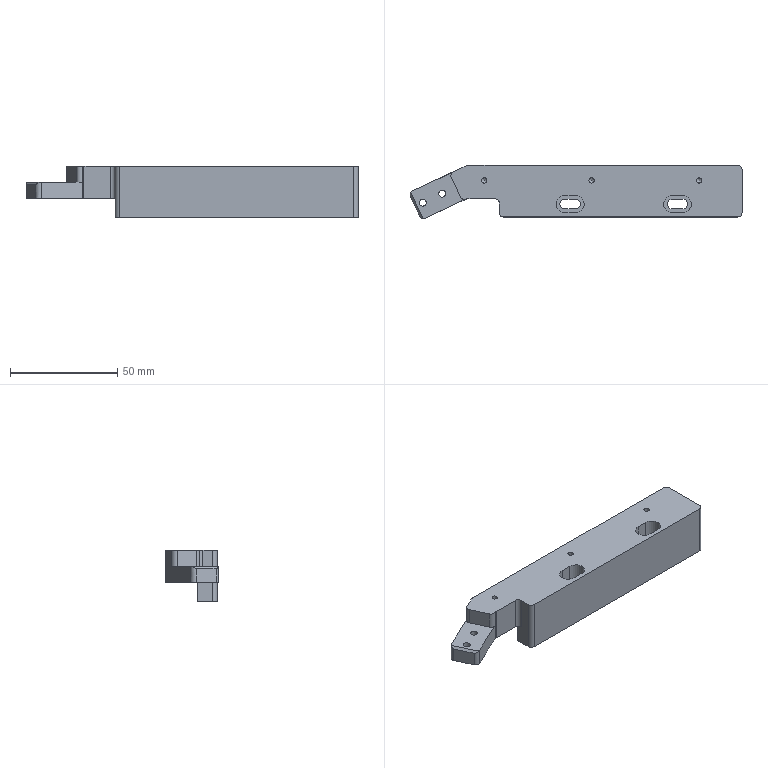Part | 1 solid | 51 faces | box 154.531 x 24.709 x 24 mm | volume 53523 mm3 | plane 25 | cylinder 23 | cone 3 | commonest cylinder face diameters 4 x10 4.5 x4 8 x4 2.459 x3 3.242 x2
STEP:
#1=CARTESIAN_POINT('',(-41.505,5.355,-8.));
#2=VERTEX_POINT('',#1);
#3=CARTESIAN_POINT('',(-42.734,5.355,-8.));
#4=DIRECTION('',(0.,0.,1.));
#5=DIRECTION('',(1.,0.,0.));
#6=AXIS2_PLACEMENT_3D('',#3,#4,#5);
#7=CIRCLE('',#6,1.23);
#8=EDGE_CURVE('',#2,#2,#7,.T.);
#9=ORIENTED_EDGE('',*,*,#8,.F.);
#10=EDGE_LOOP('',(#9));
#11=FACE_BOUND('',#10,.T.);
#12=CARTESIAN_POINT('',(-43.964,5.355,0.));
#13=VERTEX_POINT('',#12);
#14=CARTESIAN_POINT('',(-42.734,5.355,0.));
#15=DIRECTION('',(0.,0.,-1.));
#16=DIRECTION('',(-1.,0.,0.));
#17=AXIS2_PLACEMENT_3D('',#14,#15,#16);
#18=CIRCLE('',#17,1.23);
#19=EDGE_CURVE('',#13,#13,#18,.T.);
#20=ORIENTED_EDGE('',*,*,#19,.F.);
#21=EDGE_LOOP('',(#20));
#22=FACE_BOUND('',#21,.T.);
#23=CARTESIAN_POINT('',(-42.734,5.355,0.));
#24=DIRECTION('',(0.,0.,-1.));
#25=DIRECTION('',(1.,0.,0.));
#26=AXIS2_PLACEMENT_3D('',#23,#24,#25);
#27=CYLINDRICAL_SURFACE('',#26,1.23);
#28=ADVANCED_FACE('',(#11,#22),#27,.F.);
#29=ORIENTED_EDGE('',*,*,#8,.T.);
#30=EDGE_LOOP('',(#29));
#31=FACE_BOUND('',#30,.T.);
#32=CARTESIAN_POINT('',(-42.734,5.355,-8.71));
#33=VERTEX_POINT('',#32);
#34=VERTEX_LOOP('',#33);
#35=FACE_BOUND('',#34,.T.);
#36=CARTESIAN_POINT('',(-42.734,5.355,-8.71));
#37=DIRECTION('',(0.,0.,1.));
#38=DIRECTION('',(1.,0.,0.));
#39=AXIS2_PLACEMENT_3D('',#36,#37,#38);
#40=CONICAL_SURFACE('',#39,0.,1.047);
#41=ADVANCED_FACE('',(#31,#35),#40,.F.);
#42=CARTESIAN_POINT('',(8.495,5.355,-8.));
#43=VERTEX_POINT('',#42);
#44=CARTESIAN_POINT('',(7.266,5.355,-8.));
#45=DIRECTION('',(0.,0.,1.));
#46=DIRECTION('',(1.,0.,0.));
#47=AXIS2_PLACEMENT_3D('',#44,#45,#46);
#48=CIRCLE('',#47,1.23);
#49=EDGE_CURVE('',#43,#43,#48,.T.);
#50=ORIENTED_EDGE('',*,*,#49,.F.);
#51=EDGE_LOOP('',(#50));
#52=FACE_BOUND('',#51,.T.);
#53=CARTESIAN_POINT('',(6.036,5.355,0.));
#54=VERTEX_POINT('',#53);
#55=CARTESIAN_POINT('',(7.266,5.355,0.));
#56=DIRECTION('',(0.,0.,-1.));
#57=DIRECTION('',(-1.,0.,0.));
#58=AXIS2_PLACEMENT_3D('',#55,#56,#57);
#59=CIRCLE('',#58,1.23);
#60=EDGE_CURVE('',#54,#54,#59,.T.);
#61=ORIENTED_EDGE('',*,*,#60,.F.);
#62=EDGE_LOOP('',(#61));
#63=FACE_BOUND('',#62,.T.);
#64=CARTESIAN_POINT('',(7.266,5.355,0.));
#65=DIRECTION('',(0.,0.,-1.));
#66=DIRECTION('',(1.,0.,0.));
#67=AXIS2_PLACEMENT_3D('',#64,#65,#66);
#68=CYLINDRICAL_SURFACE('',#67,1.23);
#69=ADVANCED_FACE('',(#52,#63),#68,.F.);
#70=ORIENTED_EDGE('',*,*,#49,.T.);
#71=EDGE_LOOP('',(#70));
#72=FACE_BOUND('',#71,.T.);
#73=CARTESIAN_POINT('',(7.266,5.355,-8.71));
#74=VERTEX_POINT('',#73);
#75=VERTEX_LOOP('',#74);
#76=FACE_BOUND('',#75,.T.);
#77=CARTESIAN_POINT('',(7.266,5.355,-8.71));
#78=DIRECTION('',(0.,0.,1.));
#79=DIRECTION('',(1.,0.,0.));
#80=AXIS2_PLACEMENT_3D('',#77,#78,#79);
#81=CONICAL_SURFACE('',#80,0.,1.047);
#82=ADVANCED_FACE('',(#72,#76),#81,.F.);
#83=CARTESIAN_POINT('',(58.495,5.355,-8.));
#84=VERTEX_POINT('',#83);
#85=CARTESIAN_POINT('',(57.266,5.355,-8.));
#86=DIRECTION('',(0.,0.,1.));
#87=DIRECTION('',(1.,0.,0.));
#88=AXIS2_PLACEMENT_3D('',#85,#86,#87);
#89=CIRCLE('',#88,1.23);
#90=EDGE_CURVE('',#84,#84,#89,.T.);
#91=ORIENTED_EDGE('',*,*,#90,.F.);
#92=EDGE_LOOP('',(#91));
#93=FACE_BOUND('',#92,.T.);
#94=CARTESIAN_POINT('',(56.036,5.355,0.));
#95=VERTEX_POINT('',#94);
#96=CARTESIAN_POINT('',(57.266,5.355,0.));
#97=DIRECTION('',(0.,0.,-1.));
#98=DIRECTION('',(-1.,0.,0.));
#99=AXIS2_PLACEMENT_3D('',#96,#97,#98);
#100=CIRCLE('',#99,1.23);
#101=EDGE_CURVE('',#95,#95,#100,.T.);
#102=ORIENTED_EDGE('',*,*,#101,.F.);
#103=EDGE_LOOP('',(#102));
#104=FACE_BOUND('',#103,.T.);
#105=CARTESIAN_POINT('',(57.266,5.355,0.));
#106=DIRECTION('',(0.,0.,-1.));
#107=DIRECTION('',(1.,0.,0.));
#108=AXIS2_PLACEMENT_3D('',#105,#106,#107);
#109=CYLINDRICAL_SURFACE('',#108,1.23);
#110=ADVANCED_FACE('',(#93,#104),#109,.F.);
#111=ORIENTED_EDGE('',*,*,#19,.T.);
#112=EDGE_LOOP('',(#111));
#113=FACE_BOUND('',#112,.T.);
#114=ORIENTED_EDGE('',*,*,#60,.T.);
#115=EDGE_LOOP('',(#114));
#116=FACE_BOUND('',#115,.T.);
#117=CARTESIAN_POINT('',(-5.234,-1.645,0.));
#118=VERTEX_POINT('',#117);
#119=CARTESIAN_POINT('',(-0.2343,-1.645,0.));
#120=VERTEX_POINT('',#119);
#121=CARTESIAN_POINT('',(-2.734,-1.645,0.));
#122=DIRECTION('',(1.,0.,0.));
#123=VECTOR('',#122,1000.);
#124=LINE('',#121,#123);
#125=EDGE_CURVE('',#118,#120,#124,.T.);
#126=ORIENTED_EDGE('',*,*,#125,.T.);
#127=CARTESIAN_POINT('',(-0.2343,-9.645,0.));
#128=VERTEX_POINT('',#127);
#129=CARTESIAN_POINT('',(-0.2343,-5.645,0.));
#130=DIRECTION('',(0.,0.,1.));
#131=DIRECTION('',(1.,0.,0.));
#132=AXIS2_PLACEMENT_3D('',#129,#130,#131);
#133=CIRCLE('',#132,4.);
#134=EDGE_CURVE('',#128,#120,#133,.T.);
#135=ORIENTED_EDGE('',*,*,#134,.F.);
#136=CARTESIAN_POINT('',(-5.234,-9.645,0.));
#137=VERTEX_POINT('',#136);
#138=CARTESIAN_POINT('',(-2.734,-9.645,0.));
#139=DIRECTION('',(-1.,0.,0.));
#140=VECTOR('',#139,1000.);
#141=LINE('',#138,#140);
#142=EDGE_CURVE('',#128,#137,#141,.T.);
#143=ORIENTED_EDGE('',*,*,#142,.T.);
#144=CARTESIAN_POINT('',(-5.234,-5.645,0.));
#145=DIRECTION('',(0.,0.,1.));
#146=DIRECTION('',(1.,0.,0.));
#147=AXIS2_PLACEMENT_3D('',#144,#145,#146);
#148=CIRCLE('',#147,4.);
#149=EDGE_CURVE('',#118,#137,#148,.T.);
#150=ORIENTED_EDGE('',*,*,#149,.F.);
#151=EDGE_LOOP('',(#126,#135,#143,#150));
#152=FACE_BOUND('',#151,.T.);
#153=CARTESIAN_POINT('',(49.766,-9.645,0.));
#154=VERTEX_POINT('',#153);
#155=CARTESIAN_POINT('',(49.766,-1.645,0.));
#156=VERTEX_POINT('',#155);
#157=CARTESIAN_POINT('',(49.766,-5.645,0.));
#158=DIRECTION('',(0.,0.,1.));
#159=DIRECTION('',(1.,0.,0.));
#160=AXIS2_PLACEMENT_3D('',#157,#158,#159);
#161=CIRCLE('',#160,4.);
#162=EDGE_CURVE('',#154,#156,#161,.T.);
#163=ORIENTED_EDGE('',*,*,#162,.F.);
#164=CARTESIAN_POINT('',(44.766,-9.645,0.));
#165=VERTEX_POINT('',#164);
#166=CARTESIAN_POINT('',(47.266,-9.645,0.));
#167=DIRECTION('',(-1.,0.,0.));
#168=VECTOR('',#167,1000.);
#169=LINE('',#166,#168);
#170=EDGE_CURVE('',#154,#165,#169,.T.);
#171=ORIENTED_EDGE('',*,*,#170,.T.);
#172=CARTESIAN_POINT('',(44.766,-1.645,0.));
#173=VERTEX_POINT('',#172);
#174=CARTESIAN_POINT('',(44.766,-5.645,0.));
#175=DIRECTION('',(0.,0.,1.));
#176=DIRECTION('',(1.,0.,0.));
#177=AXIS2_PLACEMENT_3D('',#174,#175,#176);
#178=CIRCLE('',#177,4.);
#179=EDGE_CURVE('',#173,#165,#178,.T.);
#180=ORIENTED_EDGE('',*,*,#179,.F.);
#181=CARTESIAN_POINT('',(47.266,-1.645,0.));
#182=DIRECTION('',(1.,0.,0.));
#183=VECTOR('',#182,1000.);
#184=LINE('',#181,#183);
#185=EDGE_CURVE('',#173,#156,#184,.T.);
#186=ORIENTED_EDGE('',*,*,#185,.T.);
#187=EDGE_LOOP('',(#163,#171,#180,#186));
#188=FACE_BOUND('',#187,.T.);
#189=ORIENTED_EDGE('',*,*,#101,.T.);
#190=EDGE_LOOP('',(#189));
#191=FACE_BOUND('',#190,.T.);
#192=CARTESIAN_POINT('',(-51.162,-3.292,0.));
#193=VERTEX_POINT('',#192);
#194=CARTESIAN_POINT('',(-53.82,-2.325,0.));
#195=VERTEX_POINT('',#194);
#196=CARTESIAN_POINT('',(-52.007,-1.48,0.));
#197=DIRECTION('',(0.,0.,-1.));
#198=DIRECTION('',(-1.,0.,0.));
#199=AXIS2_PLACEMENT_3D('',#196,#197,#198);
#200=CIRCLE('',#199,2.);
#201=EDGE_CURVE('',#193,#195,#200,.T.);
#202=ORIENTED_EDGE('',*,*,#201,.F.);
#203=CARTESIAN_POINT('',(-51.136,-3.28,0.));
#204=VERTEX_POINT('',#203);
#205=CARTESIAN_POINT('',(-51.149,-3.286,0.));
#206=DIRECTION('',(-0.9063,-0.4226,0.));
#207=VECTOR('',#206,1000.);
#208=LINE('',#205,#207);
#209=EDGE_CURVE('',#204,#193,#208,.T.);
#210=ORIENTED_EDGE('',*,*,#209,.F.);
#211=CARTESIAN_POINT('',(-50.291,-3.093,0.));
#212=VERTEX_POINT('',#211);
#213=CARTESIAN_POINT('',(-50.291,-5.093,0.));
#214=DIRECTION('',(0.,0.,-1.));
#215=DIRECTION('',(-1.,0.,0.));
#216=AXIS2_PLACEMENT_3D('',#213,#214,#215);
#217=CIRCLE('',#216,2.);
#218=EDGE_CURVE('',#204,#212,#217,.T.);
#219=ORIENTED_EDGE('',*,*,#218,.T.);
#220=CARTESIAN_POINT('',(-37.734,-3.093,0.));
#221=VERTEX_POINT('',#220);
#222=CARTESIAN_POINT('',(-44.013,-3.093,0.));
#223=DIRECTION('',(1.,0.,0.));
#224=VECTOR('',#223,1000.);
#225=LINE('',#222,#224);
#226=EDGE_CURVE('',#212,#221,#225,.T.);
#227=ORIENTED_EDGE('',*,*,#226,.T.);
#228=CARTESIAN_POINT('',(-35.734,-5.093,0.));
#229=VERTEX_POINT('',#228);
#230=CARTESIAN_POINT('',(-37.734,-5.093,0.));
#231=DIRECTION('',(0.,0.,1.));
#232=DIRECTION('',(1.,0.,0.));
#233=AXIS2_PLACEMENT_3D('',#230,#231,#232);
#234=CIRCLE('',#233,2.);
#235=EDGE_CURVE('',#229,#221,#234,.T.);
#236=ORIENTED_EDGE('',*,*,#235,.F.);
#237=CARTESIAN_POINT('',(-35.734,-9.645,0.));
#238=VERTEX_POINT('',#237);
#239=CARTESIAN_POINT('',(-35.734,-5.093,0.));
#240=CARTESIAN_POINT('',(-35.734,-9.645,0.));
#241=B_SPLINE_CURVE_WITH_KNOTS('',1,(#239,#240),.UNSPECIFIED.,.F.,.F.,(2,2),(2.,6.553),.UNSPECIFIED.);
#242=EDGE_CURVE('',#229,#238,#241,.T.);
#243=ORIENTED_EDGE('',*,*,#242,.T.);
#244=CARTESIAN_POINT('',(-33.734,-11.645,0.));
#245=VERTEX_POINT('',#244);
#246=CARTESIAN_POINT('',(-33.734,-9.645,0.));
#247=DIRECTION('',(0.,0.,-1.));
#248=DIRECTION('',(-1.,0.,0.));
#249=AXIS2_PLACEMENT_3D('',#246,#247,#248);
#250=CIRCLE('',#249,2.);
#251=EDGE_CURVE('',#245,#238,#250,.T.);
#252=ORIENTED_EDGE('',*,*,#251,.F.);
#253=CARTESIAN_POINT('',(75.266,-11.645,0.));
#254=VERTEX_POINT('',#253);
#255=CARTESIAN_POINT('',(20.766,-11.645,0.));
#256=DIRECTION('',(-1.,0.,0.));
#257=VECTOR('',#256,1000.);
#258=LINE('',#255,#257);
#259=EDGE_CURVE('',#254,#245,#258,.T.);
#260=ORIENTED_EDGE('',*,*,#259,.F.);
#261=CARTESIAN_POINT('',(77.266,-9.645,0.));
#262=VERTEX_POINT('',#261);
#263=CARTESIAN_POINT('',(75.266,-9.645,0.));
#264=DIRECTION('',(0.,0.,-1.));
#265=DIRECTION('',(-1.,0.,0.));
#266=AXIS2_PLACEMENT_3D('',#263,#264,#265);
#267=CIRCLE('',#266,2.);
#268=EDGE_CURVE('',#262,#254,#267,.T.);
#269=ORIENTED_EDGE('',*,*,#268,.F.);
#270=CARTESIAN_POINT('',(77.266,10.355,0.));
#271=VERTEX_POINT('',#270);
#272=CARTESIAN_POINT('',(77.266,0.3545,0.));
#273=DIRECTION('',(0.,-1.,0.));
#274=VECTOR('',#273,1000.);
#275=LINE('',#272,#274);
#276=EDGE_CURVE('',#271,#262,#275,.T.);
#277=ORIENTED_EDGE('',*,*,#276,.F.);
#278=CARTESIAN_POINT('',(75.266,12.355,0.));
#279=VERTEX_POINT('',#278);
#280=CARTESIAN_POINT('',(75.266,10.355,0.));
#281=DIRECTION('',(0.,0.,1.));
#282=DIRECTION('',(1.,0.,0.));
#283=AXIS2_PLACEMENT_3D('',#280,#281,#282);
#284=CIRCLE('',#283,2.);
#285=EDGE_CURVE('',#271,#279,#284,.T.);
#286=ORIENTED_EDGE('',*,*,#285,.T.);
#287=CARTESIAN_POINT('',(-50.291,12.355,0.));
#288=VERTEX_POINT('',#287);
#289=CARTESIAN_POINT('',(12.487,12.355,0.));
#290=DIRECTION('',(-1.,0.,0.));
#291=VECTOR('',#290,1000.);
#292=LINE('',#289,#291);
#293=EDGE_CURVE('',#279,#288,#292,.T.);
#294=ORIENTED_EDGE('',*,*,#293,.T.);
#295=CARTESIAN_POINT('',(-51.136,12.167,0.));
#296=VERTEX_POINT('',#295);
#297=CARTESIAN_POINT('',(-50.291,10.355,0.));
#298=DIRECTION('',(0.,0.,-1.));
#299=DIRECTION('',(-1.,0.,0.));
#300=AXIS2_PLACEMENT_3D('',#297,#298,#299);
#301=CIRCLE('',#300,2.);
#302=EDGE_CURVE('',#296,#288,#301,.T.);
#303=ORIENTED_EDGE('',*,*,#302,.F.);
#304=CARTESIAN_POINT('',(-57.078,9.396,0.));
#305=VERTEX_POINT('',#304);
#306=CARTESIAN_POINT('',(-54.107,10.782,0.));
#307=DIRECTION('',(0.9063,0.4226,0.));
#308=VECTOR('',#307,1000.);
#309=LINE('',#306,#308);
#310=EDGE_CURVE('',#305,#296,#309,.T.);
#311=ORIENTED_EDGE('',*,*,#310,.F.);
#312=CARTESIAN_POINT('',(-58.046,6.738,0.));
#313=VERTEX_POINT('',#312);
#314=CARTESIAN_POINT('',(-56.233,7.584,0.));
#315=DIRECTION('',(0.,0.,-1.));
#316=DIRECTION('',(-1.,0.,0.));
#317=AXIS2_PLACEMENT_3D('',#314,#315,#316);
#318=CIRCLE('',#317,2.);
#319=EDGE_CURVE('',#313,#305,#318,.T.);
#320=ORIENTED_EDGE('',*,*,#319,.F.);
#321=CARTESIAN_POINT('',(-55.933,2.207,0.));
#322=DIRECTION('',(0.4226,-0.9063,0.));
#323=VECTOR('',#322,1000.);
#324=LINE('',#321,#323);
#325=EDGE_CURVE('',#313,#195,#324,.T.);
#326=ORIENTED_EDGE('',*,*,#325,.T.);
#327=EDGE_LOOP('',(#202,#210,#219,#227,#236,#243,#252,#260,#269,#277,#286,#294,#303,#311,#320,#326));
#328=FACE_BOUND('',#327,.T.);
#329=CARTESIAN_POINT('',(77.266,12.355,0.));
#330=DIRECTION('',(0.,0.,-1.));
#331=DIRECTION('',(0.,-1.,0.));
#332=AXIS2_PLACEMENT_3D('',#329,#330,#331);
#333=PLANE('',#332);
#334=ADVANCED_FACE('',(#113,#116,#152,#188,#191,#328),#333,.F.);
#335=CARTESIAN_POINT('',(-53.82,-2.325,-7.5));
#336=VERTEX_POINT('',#335);
#337=CARTESIAN_POINT('',(-53.82,-2.325,-7.5));
#338=DIRECTION('',(0.,0.,-1.));
#339=VECTOR('',#338,1000.);
#340=LINE('',#337,#339);
#341=EDGE_CURVE('',#195,#336,#340,.T.);
#342=ORIENTED_EDGE('',*,*,#341,.F.);
#343=ORIENTED_EDGE('',*,*,#325,.F.);
#344=CARTESIAN_POINT('',(-58.046,6.738,-7.5));
#345=VERTEX_POINT('',#344);
#346=CARTESIAN_POINT('',(-58.046,6.738,-7.5));
#347=DIRECTION('',(0.,0.,-1.));
#348=VECTOR('',#347,1000.);
#349=LINE('',#346,#348);
#350=EDGE_CURVE('',#313,#345,#349,.T.);
#351=ORIENTED_EDGE('',*,*,#350,.T.);
#352=CARTESIAN_POINT('',(-55.933,2.207,-7.5));
#353=DIRECTION('',(0.4226,-0.9063,0.));
#354=VECTOR('',#353,1000.);
#355=LINE('',#352,#354);
#356=EDGE_CURVE('',#345,#336,#355,.T.);
#357=ORIENTED_EDGE('',*,*,#356,.T.);
#358=EDGE_LOOP('',(#342,#343,#351,#357));
#359=FACE_BOUND('',#358,.T.);
#360=CARTESIAN_POINT('',(-58.891,8.551,0.));
#361=DIRECTION('',(0.9063,0.4226,0.));
#362=DIRECTION('',(0.4226,-0.9063,0.));
#363=AXIS2_PLACEMENT_3D('',#360,#361,#362);
#364=PLANE('',#363);
#365=ADVANCED_FACE('',(#359),#364,.F.);
#366=CARTESIAN_POINT('',(-57.078,9.396,-7.5));
#367=VERTEX_POINT('',#366);
#368=CARTESIAN_POINT('',(-56.233,7.584,-7.5));
#369=DIRECTION('',(0.,0.,1.));
#370=DIRECTION('',(1.,0.,0.));
#371=AXIS2_PLACEMENT_3D('',#368,#369,#370);
#372=CIRCLE('',#371,2.);
#373=EDGE_CURVE('',#367,#345,#372,.T.);
#374=ORIENTED_EDGE('',*,*,#373,.T.);
#375=ORIENTED_EDGE('',*,*,#350,.F.);
#376=ORIENTED_EDGE('',*,*,#319,.T.);
#377=CARTESIAN_POINT('',(-57.078,9.396,-3.75));
#378=DIRECTION('',(0.,0.,-1.));
#379=VECTOR('',#378,1000.);
#380=LINE('',#377,#379);
#381=EDGE_CURVE('',#305,#367,#380,.T.);
#382=ORIENTED_EDGE('',*,*,#381,.T.);
#383=EDGE_LOOP('',(#374,#375,#376,#382));
#384=FACE_BOUND('',#383,.T.);
#385=CARTESIAN_POINT('',(-56.233,7.584,-7.5));
#386=DIRECTION('',(0.,0.,-1.));
#387=DIRECTION('',(-0.9063,-0.4226,0.));
#388=AXIS2_PLACEMENT_3D('',#385,#386,#387);
#389=CYLINDRICAL_SURFACE('',#388,2.);
#390=ADVANCED_FACE('',(#384),#389,.T.);
#391=ORIENTED_EDGE('',*,*,#302,.T.);
#392=CARTESIAN_POINT('',(-50.291,12.355,-15.));
#393=VERTEX_POINT('',#392);
#394=CARTESIAN_POINT('',(-50.291,12.355,-7.5));
#395=DIRECTION('',(0.,0.,-1.));
#396=VECTOR('',#395,1000.);
#397=LINE('',#394,#396);
#398=EDGE_CURVE('',#288,#393,#397,.T.);
#399=ORIENTED_EDGE('',*,*,#398,.T.);
#400=CARTESIAN_POINT('',(-51.136,12.167,-15.));
#401=VERTEX_POINT('',#400);
#402=CARTESIAN_POINT('',(-50.291,10.355,-15.));
#403=DIRECTION('',(0.,0.,1.));
#404=DIRECTION('',(1.,0.,0.));
#405=AXIS2_PLACEMENT_3D('',#402,#403,#404);
#406=CIRCLE('',#405,2.);
#407=EDGE_CURVE('',#393,#401,#406,.T.);
#408=ORIENTED_EDGE('',*,*,#407,.T.);
#409=CARTESIAN_POINT('',(-51.136,12.167,-7.5));
#410=DIRECTION('',(0.,0.,-1.));
#411=VECTOR('',#410,1000.);
#412=LINE('',#409,#411);
#413=EDGE_CURVE('',#296,#401,#412,.T.);
#414=ORIENTED_EDGE('',*,*,#413,.F.);
#415=EDGE_LOOP('',(#391,#399,#408,#414));
#416=FACE_BOUND('',#415,.T.);
#417=CARTESIAN_POINT('',(-50.291,10.355,-7.5));
#418=DIRECTION('',(0.,0.,-1.));
#419=DIRECTION('',(-0.4226,0.9063,0.));
#420=AXIS2_PLACEMENT_3D('',#417,#418,#419);
#421=CYLINDRICAL_SURFACE('',#420,2.);
#422=ADVANCED_FACE('',(#416),#421,.T.);
#423=ORIENTED_EDGE('',*,*,#285,.F.);
#424=CARTESIAN_POINT('',(77.266,10.355,-15.));
#425=VERTEX_POINT('',#424);
#426=CARTESIAN_POINT('',(77.266,10.355,-7.5));
#427=DIRECTION('',(0.,0.,1.));
#428=VECTOR('',#427,1000.);
#429=LINE('',#426,#428);
#430=EDGE_CURVE('',#425,#271,#429,.T.);
#431=ORIENTED_EDGE('',*,*,#430,.F.);
#432=CARTESIAN_POINT('',(75.266,12.355,-15.));
#433=VERTEX_POINT('',#432);
#434=CARTESIAN_POINT('',(75.266,10.355,-15.));
#435=DIRECTION('',(0.,0.,1.));
#436=DIRECTION('',(1.,0.,0.));
#437=AXIS2_PLACEMENT_3D('',#434,#435,#436);
#438=CIRCLE('',#437,2.);
#439=EDGE_CURVE('',#425,#433,#438,.T.);
#440=ORIENTED_EDGE('',*,*,#439,.T.);
#441=CARTESIAN_POINT('',(75.266,12.355,-7.5));
#442=DIRECTION('',(0.,0.,1.));
#443=VECTOR('',#442,1000.);
#444=LINE('',#441,#443);
#445=EDGE_CURVE('',#433,#279,#444,.T.);
#446=ORIENTED_EDGE('',*,*,#445,.T.);
#447=EDGE_LOOP('',(#423,#431,#440,#446));
#448=FACE_BOUND('',#447,.T.);
#449=CARTESIAN_POINT('',(75.266,10.355,-12.));
#450=DIRECTION('',(0.,0.,1.));
#451=DIRECTION('',(1.,0.,0.));
#452=AXIS2_PLACEMENT_3D('',#449,#450,#451);
#453=CYLINDRICAL_SURFACE('',#452,2.);
#454=ADVANCED_FACE('',(#448),#453,.T.);
#455=CARTESIAN_POINT('',(77.266,-9.645,-24.));
#456=VERTEX_POINT('',#455);
#457=CARTESIAN_POINT('',(77.266,-2.645,-24.));
#458=VERTEX_POINT('',#457);
#459=CARTESIAN_POINT('',(77.266,-6.145,-24.));
#460=DIRECTION('',(0.,1.,0.));
#461=VECTOR('',#460,1000.);
#462=LINE('',#459,#461);
#463=EDGE_CURVE('',#456,#458,#462,.T.);
#464=ORIENTED_EDGE('',*,*,#463,.T.);
#465=CARTESIAN_POINT('',(77.266,-2.645,-15.));
#466=VERTEX_POINT('',#465);
#467=CARTESIAN_POINT('',(77.266,-2.645,-19.5));
#468=DIRECTION('',(0.,0.,-1.));
#469=VECTOR('',#468,1000.);
#470=LINE('',#467,#469);
#471=EDGE_CURVE('',#466,#458,#470,.T.);
#472=ORIENTED_EDGE('',*,*,#471,.F.);
#473=CARTESIAN_POINT('',(77.266,3.855,-15.));
#474=DIRECTION('',(0.,1.,0.));
#475=VECTOR('',#474,1000.);
#476=LINE('',#473,#475);
#477=EDGE_CURVE('',#466,#425,#476,.T.);
#478=ORIENTED_EDGE('',*,*,#477,.T.);
#479=ORIENTED_EDGE('',*,*,#430,.T.);
#480=ORIENTED_EDGE('',*,*,#276,.T.);
#481=CARTESIAN_POINT('',(77.266,-9.645,-12.));
#482=DIRECTION('',(0.,0.,-1.));
#483=VECTOR('',#482,1000.);
#484=LINE('',#481,#483);
#485=EDGE_CURVE('',#262,#456,#484,.T.);
#486=ORIENTED_EDGE('',*,*,#485,.T.);
#487=EDGE_LOOP('',(#464,#472,#478,#479,#480,#486));
#488=FACE_BOUND('',#487,.T.);
#489=CARTESIAN_POINT('',(77.266,-11.645,-24.));
#490=DIRECTION('',(1.,0.,0.));
#491=DIRECTION('',(0.,1.,0.));
#492=AXIS2_PLACEMENT_3D('',#489,#490,#491);
#493=PLANE('',#492);
#494=ADVANCED_FACE('',(#488),#493,.T.);
#495=CARTESIAN_POINT('',(75.266,-11.645,-24.));
#496=VERTEX_POINT('',#495);
#497=CARTESIAN_POINT('',(75.266,-9.645,-24.));
#498=DIRECTION('',(0.,0.,1.));
#499=DIRECTION('',(1.,0.,0.));
#500=AXIS2_PLACEMENT_3D('',#497,#498,#499);
#501=CIRCLE('',#500,2.);
#502=EDGE_CURVE('',#496,#456,#501,.T.);
#503=ORIENTED_EDGE('',*,*,#502,.T.);
#504=ORIENTED_EDGE('',*,*,#485,.F.);
#505=ORIENTED_EDGE('',*,*,#268,.T.);
#506=CARTESIAN_POINT('',(75.266,-11.645,-12.));
#507=DIRECTION('',(0.,0.,-1.));
#508=VECTOR('',#507,1000.);
#509=LINE('',#506,#508);
#510=EDGE_CURVE('',#254,#496,#509,.T.);
#511=ORIENTED_EDGE('',*,*,#510,.T.);
#512=EDGE_LOOP('',(#503,#504,#505,#511));
#513=FACE_BOUND('',#512,.T.);
#514=CARTESIAN_POINT('',(75.266,-9.645,-12.));
#515=DIRECTION('',(0.,0.,-1.));
#516=DIRECTION('',(1.,0.,0.));
#517=AXIS2_PLACEMENT_3D('',#514,#515,#516);
#518=CYLINDRICAL_SURFACE('',#517,2.);
#519=ADVANCED_FACE('',(#513),#518,.T.);
#520=CARTESIAN_POINT('',(-33.734,-11.645,-24.));
#521=VERTEX_POINT('',#520);
#522=CARTESIAN_POINT('',(-33.734,-11.645,-12.));
#523=DIRECTION('',(0.,0.,-1.));
#524=VECTOR('',#523,1000.);
#525=LINE('',#522,#524);
#526=EDGE_CURVE('',#245,#521,#525,.T.);
#527=ORIENTED_EDGE('',*,*,#526,.T.);
#528=CARTESIAN_POINT('',(20.766,-11.645,-24.));
#529=DIRECTION('',(-1.,0.,0.));
#530=VECTOR('',#529,1000.);
#531=LINE('',#528,#530);
#532=EDGE_CURVE('',#496,#521,#531,.T.);
#533=ORIENTED_EDGE('',*,*,#532,.F.);
#534=ORIENTED_EDGE('',*,*,#510,.F.);
#535=ORIENTED_EDGE('',*,*,#259,.T.);
#536=EDGE_LOOP('',(#527,#533,#534,#535));
#537=FACE_BOUND('',#536,.T.);
#538=CARTESIAN_POINT('',(77.266,-11.645,0.));
#539=DIRECTION('',(0.,1.,0.));
#540=DIRECTION('',(0.,0.,-1.));
#541=AXIS2_PLACEMENT_3D('',#538,#539,#540);
#542=PLANE('',#541);
#543=ADVANCED_FACE('',(#537),#542,.F.);
#544=ORIENTED_EDGE('',*,*,#251,.T.);
#545=CARTESIAN_POINT('',(-35.734,-9.645,-24.));
#546=VERTEX_POINT('',#545);
#547=CARTESIAN_POINT('',(-35.734,-9.645,-12.));
#548=DIRECTION('',(0.,0.,-1.));
#549=VECTOR('',#548,1000.);
#550=LINE('',#547,#549);
#551=EDGE_CURVE('',#238,#546,#550,.T.);
#552=ORIENTED_EDGE('',*,*,#551,.T.);
#553=CARTESIAN_POINT('',(-33.734,-9.645,-24.));
#554=DIRECTION('',(0.,0.,1.));
#555=DIRECTION('',(1.,0.,0.));
#556=AXIS2_PLACEMENT_3D('',#553,#554,#555);
#557=CIRCLE('',#556,2.);
#558=EDGE_CURVE('',#546,#521,#557,.T.);
#559=ORIENTED_EDGE('',*,*,#558,.T.);
#560=ORIENTED_EDGE('',*,*,#526,.F.);
#561=EDGE_LOOP('',(#544,#552,#559,#560));
#562=FACE_BOUND('',#561,.T.);
#563=CARTESIAN_POINT('',(-33.734,-9.645,-12.));
#564=DIRECTION('',(0.,0.,-1.));
#565=DIRECTION('',(0.,-1.,0.));
#566=AXIS2_PLACEMENT_3D('',#563,#564,#565);
#567=CYLINDRICAL_SURFACE('',#566,2.);
#568=ADVANCED_FACE('',(#562),#567,.T.);
#569=ORIENTED_EDGE('',*,*,#242,.F.);
#570=CARTESIAN_POINT('',(-35.734,-5.093,-15.));
#571=VERTEX_POINT('',#570);
#572=CARTESIAN_POINT('',(-35.734,-5.093,-12.));
#573=DIRECTION('',(0.,0.,1.));
#574=VECTOR('',#573,1000.);
#575=LINE('',#572,#574);
#576=EDGE_CURVE('',#571,#229,#575,.T.);
#577=ORIENTED_EDGE('',*,*,#576,.F.);
#578=CARTESIAN_POINT('',(-35.734,-2.645,-15.));
#579=VERTEX_POINT('',#578);
#580=CARTESIAN_POINT('',(-35.734,-3.869,-15.));
#581=DIRECTION('',(0.,-1.,0.));
#582=VECTOR('',#581,1000.);
#583=LINE('',#580,#582);
#584=EDGE_CURVE('',#579,#571,#583,.T.);
#585=ORIENTED_EDGE('',*,*,#584,.F.);
#586=CARTESIAN_POINT('',(-35.734,-2.645,-24.));
#587=VERTEX_POINT('',#586);
#588=CARTESIAN_POINT('',(-35.734,-2.645,-19.5));
#589=DIRECTION('',(0.,0.,1.));
#590=VECTOR('',#589,1000.);
#591=LINE('',#588,#590);
#592=EDGE_CURVE('',#587,#579,#591,.T.);
#593=ORIENTED_EDGE('',*,*,#592,.F.);
#594=CARTESIAN_POINT('',(-35.734,-6.145,-24.));
#595=DIRECTION('',(0.,1.,0.));
#596=VECTOR('',#595,1000.);
#597=LINE('',#594,#596);
#598=EDGE_CURVE('',#546,#587,#597,.T.);
#599=ORIENTED_EDGE('',*,*,#598,.F.);
#600=ORIENTED_EDGE('',*,*,#551,.F.);
#601=EDGE_LOOP('',(#569,#577,#585,#593,#599,#600));
#602=FACE_BOUND('',#601,.T.);
#603=CARTESIAN_POINT('',(-35.734,-11.645,-24.));
#604=DIRECTION('',(-1.,0.,0.));
#605=DIRECTION('',(0.,-1.,0.));
#606=AXIS2_PLACEMENT_3D('',#603,#604,#605);
#607=PLANE('',#606);
#608=ADVANCED_FACE('',(#602),#607,.T.);
#609=CARTESIAN_POINT('',(-51.162,-3.292,-7.5));
#610=VERTEX_POINT('',#609);
#611=CARTESIAN_POINT('',(-52.007,-1.48,-7.5));
#612=DIRECTION('',(0.,0.,1.));
#613=DIRECTION('',(1.,0.,0.));
#614=AXIS2_PLACEMENT_3D('',#611,#612,#613);
#615=CIRCLE('',#614,2.);
#616=EDGE_CURVE('',#336,#610,#615,.T.);
#617=ORIENTED_EDGE('',*,*,#616,.T.);
#618=CARTESIAN_POINT('',(-51.162,-3.292,-3.75));
#619=DIRECTION('',(0.,0.,-1.));
#620=VECTOR('',#619,1000.);
#621=LINE('',#618,#620);
#622=EDGE_CURVE('',#193,#610,#621,.T.);
#623=ORIENTED_EDGE('',*,*,#622,.F.);
#624=ORIENTED_EDGE('',*,*,#201,.T.);
#625=ORIENTED_EDGE('',*,*,#341,.T.);
#626=EDGE_LOOP('',(#617,#623,#624,#625));
#627=FACE_BOUND('',#626,.T.);
#628=CARTESIAN_POINT('',(-52.007,-1.48,-7.5));
#629=DIRECTION('',(0.,0.,-1.));
#630=DIRECTION('',(0.4226,-0.9063,0.));
#631=AXIS2_PLACEMENT_3D('',#628,#629,#630);
#632=CYLINDRICAL_SURFACE('',#631,2.);
#633=ADVANCED_FACE('',(#627),#632,.T.);
#634=CARTESIAN_POINT('',(44.766,-1.645,-10.));
#635=VERTEX_POINT('',#634);
#636=CARTESIAN_POINT('',(49.766,-1.645,-10.));
#637=VERTEX_POINT('',#636);
#638=CARTESIAN_POINT('',(47.266,-1.645,-10.));
#639=DIRECTION('',(1.,0.,0.));
#640=VECTOR('',#639,1000.);
#641=LINE('',#638,#640);
#642=EDGE_CURVE('',#635,#637,#641,.T.);
#643=ORIENTED_EDGE('',*,*,#642,.T.);
#644=CARTESIAN_POINT('',(49.766,-1.645,-5.));
#645=DIRECTION('',(0.,0.,1.));
#646=VECTOR('',#645,1000.);
#647=LINE('',#644,#646);
#648=EDGE_CURVE('',#637,#156,#647,.T.);
#649=ORIENTED_EDGE('',*,*,#648,.T.);
#650=ORIENTED_EDGE('',*,*,#185,.F.);
#651=CARTESIAN_POINT('',(44.766,-1.645,-5.));
#652=DIRECTION('',(0.,0.,1.));
#653=VECTOR('',#652,1000.);
#654=LINE('',#651,#653);
#655=EDGE_CURVE('',#635,#173,#654,.T.);
#656=ORIENTED_EDGE('',*,*,#655,.F.);
#657=EDGE_LOOP('',(#643,#649,#650,#656));
#658=FACE_BOUND('',#657,.T.);
#659=CARTESIAN_POINT('',(44.766,-1.645,0.));
#660=DIRECTION('',(0.,1.,0.));
#661=DIRECTION('',(1.,0.,0.));
#662=AXIS2_PLACEMENT_3D('',#659,#660,#661);
#663=PLANE('',#662);
#664=ADVANCED_FACE('',(#658),#663,.F.);
#665=ORIENTED_EDGE('',*,*,#655,.T.);
#666=ORIENTED_EDGE('',*,*,#179,.T.);
#667=CARTESIAN_POINT('',(44.766,-9.645,-10.));
#668=VERTEX_POINT('',#667);
#669=CARTESIAN_POINT('',(44.766,-9.645,-5.));
#670=DIRECTION('',(0.,0.,-1.));
#671=VECTOR('',#670,1000.);
#672=LINE('',#669,#671);
#673=EDGE_CURVE('',#165,#668,#672,.T.);
#674=ORIENTED_EDGE('',*,*,#673,.T.);
#675=CARTESIAN_POINT('',(44.766,-5.645,-10.));
#676=DIRECTION('',(0.,0.,-1.));
#677=DIRECTION('',(-1.,0.,0.));
#678=AXIS2_PLACEMENT_3D('',#675,#676,#677);
#679=CIRCLE('',#678,4.);
#680=EDGE_CURVE('',#668,#635,#679,.T.);
#681=ORIENTED_EDGE('',*,*,#680,.T.);
#682=EDGE_LOOP('',(#665,#666,#674,#681));
#683=FACE_BOUND('',#682,.T.);
#684=CARTESIAN_POINT('',(44.766,-5.645,-5.));
#685=DIRECTION('',(0.,0.,1.));
#686=DIRECTION('',(0.,1.,0.));
#687=AXIS2_PLACEMENT_3D('',#684,#685,#686);
#688=CYLINDRICAL_SURFACE('',#687,4.);
#689=ADVANCED_FACE('',(#683),#688,.F.);
#690=ORIENTED_EDGE('',*,*,#170,.F.);
#691=CARTESIAN_POINT('',(49.766,-9.645,-10.));
#692=VERTEX_POINT('',#691);
#693=CARTESIAN_POINT('',(49.766,-9.645,-5.));
#694=DIRECTION('',(0.,0.,1.));
#695=VECTOR('',#694,1000.);
#696=LINE('',#693,#695);
#697=EDGE_CURVE('',#692,#154,#696,.T.);
#698=ORIENTED_EDGE('',*,*,#697,.F.);
#699=CARTESIAN_POINT('',(47.266,-9.645,-10.));
#700=DIRECTION('',(-1.,0.,0.));
#701=VECTOR('',#700,1000.);
#702=LINE('',#699,#701);
#703=EDGE_CURVE('',#692,#668,#702,.T.);
#704=ORIENTED_EDGE('',*,*,#703,.T.);
#705=ORIENTED_EDGE('',*,*,#673,.F.);
#706=EDGE_LOOP('',(#690,#698,#704,#705));
#707=FACE_BOUND('',#706,.T.);
#708=CARTESIAN_POINT('',(49.766,-9.645,0.));
#709=DIRECTION('',(0.,-1.,0.));
#710=DIRECTION('',(-1.,0.,0.));
#711=AXIS2_PLACEMENT_3D('',#708,#709,#710);
#712=PLANE('',#711);
#713=ADVANCED_FACE('',(#707),#712,.F.);
#714=ORIENTED_EDGE('',*,*,#697,.T.);
#715=ORIENTED_EDGE('',*,*,#162,.T.);
#716=ORIENTED_EDGE('',*,*,#648,.F.);
#717=CARTESIAN_POINT('',(49.766,-5.645,-10.));
#718=DIRECTION('',(0.,0.,-1.));
#719=DIRECTION('',(-1.,0.,0.));
#720=AXIS2_PLACEMENT_3D('',#717,#718,#719);
#721=CIRCLE('',#720,4.);
#722=EDGE_CURVE('',#637,#692,#721,.T.);
#723=ORIENTED_EDGE('',*,*,#722,.T.);
#724=EDGE_LOOP('',(#714,#715,#716,#723));
#725=FACE_BOUND('',#724,.T.);
#726=CARTESIAN_POINT('',(49.766,-5.645,-5.));
#727=DIRECTION('',(0.,0.,1.));
#728=DIRECTION('',(0.,-1.,0.));
#729=AXIS2_PLACEMENT_3D('',#726,#727,#728);
#730=CYLINDRICAL_SURFACE('',#729,4.);
#731=ADVANCED_FACE('',(#725),#730,.F.);
#732=CARTESIAN_POINT('',(-5.234,-1.645,-10.));
#733=VERTEX_POINT('',#732);
#734=CARTESIAN_POINT('',(-5.234,-1.645,-5.));
#735=DIRECTION('',(0.,0.,-1.));
#736=VECTOR('',#735,1000.);
#737=LINE('',#734,#736);
#738=EDGE_CURVE('',#118,#733,#737,.T.);
#739=ORIENTED_EDGE('',*,*,#738,.F.);
#740=ORIENTED_EDGE('',*,*,#149,.T.);
#741=CARTESIAN_POINT('',(-5.234,-9.645,-10.));
#742=VERTEX_POINT('',#741);
#743=CARTESIAN_POINT('',(-5.234,-9.645,-5.));
#744=DIRECTION('',(0.,0.,-1.));
#745=VECTOR('',#744,1000.);
#746=LINE('',#743,#745);
#747=EDGE_CURVE('',#137,#742,#746,.T.);
#748=ORIENTED_EDGE('',*,*,#747,.T.);
#749=CARTESIAN_POINT('',(-5.234,-5.645,-10.));
#750=DIRECTION('',(0.,0.,-1.));
#751=DIRECTION('',(-1.,0.,0.));
#752=AXIS2_PLACEMENT_3D('',#749,#750,#751);
#753=CIRCLE('',#752,4.);
#754=EDGE_CURVE('',#742,#733,#753,.T.);
#755=ORIENTED_EDGE('',*,*,#754,.T.);
#756=EDGE_LOOP('',(#739,#740,#748,#755));
#757=FACE_BOUND('',#756,.T.);
#758=CARTESIAN_POINT('',(-5.234,-5.645,-5.));
#759=DIRECTION('',(0.,0.,1.));
#760=DIRECTION('',(0.,1.,0.));
#761=AXIS2_PLACEMENT_3D('',#758,#759,#760);
#762=CYLINDRICAL_SURFACE('',#761,4.);
#763=ADVANCED_FACE('',(#757),#762,.F.);
#764=ORIENTED_EDGE('',*,*,#142,.F.);
#765=CARTESIAN_POINT('',(-0.2343,-9.645,-10.));
#766=VERTEX_POINT('',#765);
#767=CARTESIAN_POINT('',(-0.2343,-9.645,-5.));
#768=DIRECTION('',(0.,0.,1.));
#769=VECTOR('',#768,1000.);
#770=LINE('',#767,#769);
#771=EDGE_CURVE('',#766,#128,#770,.T.);
#772=ORIENTED_EDGE('',*,*,#771,.F.);
#773=CARTESIAN_POINT('',(-2.734,-9.645,-10.));
#774=DIRECTION('',(-1.,0.,0.));
#775=VECTOR('',#774,1000.);
#776=LINE('',#773,#775);
#777=EDGE_CURVE('',#766,#742,#776,.T.);
#778=ORIENTED_EDGE('',*,*,#777,.T.);
#779=ORIENTED_EDGE('',*,*,#747,.F.);
#780=EDGE_LOOP('',(#764,#772,#778,#779));
#781=FACE_BOUND('',#780,.T.);
#782=CARTESIAN_POINT('',(49.766,-9.645,0.));
#783=DIRECTION('',(0.,-1.,0.));
#784=DIRECTION('',(-1.,0.,0.));
#785=AXIS2_PLACEMENT_3D('',#782,#783,#784);
#786=PLANE('',#785);
#787=ADVANCED_FACE('',(#781),#786,.F.);
#788=ORIENTED_EDGE('',*,*,#771,.T.);
#789=ORIENTED_EDGE('',*,*,#134,.T.);
#790=CARTESIAN_POINT('',(-0.2343,-1.645,-10.));
#791=VERTEX_POINT('',#790);
#792=CARTESIAN_POINT('',(-0.2343,-1.645,-5.));
#793=DIRECTION('',(0.,0.,-1.));
#794=VECTOR('',#793,1000.);
#795=LINE('',#792,#794);
#796=EDGE_CURVE('',#120,#791,#795,.T.);
#797=ORIENTED_EDGE('',*,*,#796,.T.);
#798=CARTESIAN_POINT('',(-0.2343,-5.645,-10.));
#799=DIRECTION('',(0.,0.,-1.));
#800=DIRECTION('',(-1.,0.,0.));
#801=AXIS2_PLACEMENT_3D('',#798,#799,#800);
#802=CIRCLE('',#801,4.);
#803=EDGE_CURVE('',#791,#766,#802,.T.);
#804=ORIENTED_EDGE('',*,*,#803,.T.);
#805=EDGE_LOOP('',(#788,#789,#797,#804));
#806=FACE_BOUND('',#805,.T.);
#807=CARTESIAN_POINT('',(-0.2343,-5.645,-5.));
#808=DIRECTION('',(0.,0.,1.));
#809=DIRECTION('',(0.,-1.,0.));
#810=AXIS2_PLACEMENT_3D('',#807,#808,#809);
#811=CYLINDRICAL_SURFACE('',#810,4.);
#812=ADVANCED_FACE('',(#806),#811,.F.);
#813=CARTESIAN_POINT('',(-2.734,-1.645,-10.));
#814=DIRECTION('',(1.,0.,0.));
#815=VECTOR('',#814,1000.);
#816=LINE('',#813,#815);
#817=EDGE_CURVE('',#733,#791,#816,.T.);
#818=ORIENTED_EDGE('',*,*,#817,.T.);
#819=ORIENTED_EDGE('',*,*,#796,.F.);
#820=ORIENTED_EDGE('',*,*,#125,.F.);
#821=ORIENTED_EDGE('',*,*,#738,.T.);
#822=EDGE_LOOP('',(#818,#819,#820,#821));
#823=FACE_BOUND('',#822,.T.);
#824=CARTESIAN_POINT('',(44.766,-1.645,0.));
#825=DIRECTION('',(0.,1.,0.));
#826=DIRECTION('',(1.,0.,0.));
#827=AXIS2_PLACEMENT_3D('',#824,#825,#826);
#828=PLANE('',#827);
#829=ADVANCED_FACE('',(#823),#828,.F.);
#830=CARTESIAN_POINT('',(-72.961,-4.978,-7.5));
#831=VERTEX_POINT('',#830);
#832=CARTESIAN_POINT('',(-71.34,-4.978,-7.5));
#833=DIRECTION('',(0.,0.,-1.));
#834=DIRECTION('',(-1.,0.,0.));
#835=AXIS2_PLACEMENT_3D('',#832,#833,#834);
#836=CIRCLE('',#835,1.621);
#837=EDGE_CURVE('',#831,#831,#836,.T.);
#838=ORIENTED_EDGE('',*,*,#837,.T.);
#839=EDGE_LOOP('',(#838));
#840=FACE_BOUND('',#839,.T.);
#841=CARTESIAN_POINT('',(-63.898,-0.7515,-7.5));
#842=VERTEX_POINT('',#841);
#843=CARTESIAN_POINT('',(-62.277,-0.7515,-7.5));
#844=DIRECTION('',(0.,0.,-1.));
#845=DIRECTION('',(-1.,0.,0.));
#846=AXIS2_PLACEMENT_3D('',#843,#844,#845);
#847=CIRCLE('',#846,1.621);
#848=EDGE_CURVE('',#842,#842,#847,.T.);
#849=ORIENTED_EDGE('',*,*,#848,.T.);
#850=EDGE_LOOP('',(#849));
#851=FACE_BOUND('',#850,.T.);
#852=CARTESIAN_POINT('',(-70.194,-12.167,-7.5));
#853=VERTEX_POINT('',#852);
#854=CARTESIAN_POINT('',(-60.678,-7.73,-7.5));
#855=DIRECTION('',(0.9063,0.4226,0.));
#856=VECTOR('',#855,1000.);
#857=LINE('',#854,#856);
#858=EDGE_CURVE('',#853,#610,#857,.T.);
#859=ORIENTED_EDGE('',*,*,#858,.T.);
#860=ORIENTED_EDGE('',*,*,#616,.F.);
#861=ORIENTED_EDGE('',*,*,#356,.F.);
#862=ORIENTED_EDGE('',*,*,#373,.F.);
#863=CARTESIAN_POINT('',(-76.111,0.5212,-7.5));
#864=VERTEX_POINT('',#863);
#865=CARTESIAN_POINT('',(-66.595,4.959,-7.5));
#866=DIRECTION('',(0.9063,0.4226,0.));
#867=VECTOR('',#866,1000.);
#868=LINE('',#865,#867);
#869=EDGE_CURVE('',#864,#367,#868,.T.);
#870=ORIENTED_EDGE('',*,*,#869,.F.);
#871=CARTESIAN_POINT('',(-76.904,-0.1443,-7.5));
#872=VERTEX_POINT('',#871);
#873=CARTESIAN_POINT('',(-75.266,-1.291,-7.5));
#874=DIRECTION('',(0.,0.,-1.));
#875=DIRECTION('',(-1.,0.,0.));
#876=AXIS2_PLACEMENT_3D('',#873,#874,#875);
#877=CIRCLE('',#876,2.);
#878=EDGE_CURVE('',#872,#864,#877,.T.);
#879=ORIENTED_EDGE('',*,*,#878,.F.);
#880=CARTESIAN_POINT('',(-71.214,-12.347,-7.5));
#881=VERTEX_POINT('',#880);
#882=CARTESIAN_POINT('',(-76.045,-1.987,-7.5));
#883=DIRECTION('',(-0.4226,0.9063,0.));
#884=VECTOR('',#883,1000.);
#885=LINE('',#882,#884);
#886=EDGE_CURVE('',#881,#872,#885,.T.);
#887=ORIENTED_EDGE('',*,*,#886,.F.);
#888=CARTESIAN_POINT('',(-71.04,-10.355,-7.5));
#889=DIRECTION('',(0.,0.,-1.));
#890=DIRECTION('',(-1.,0.,0.));
#891=AXIS2_PLACEMENT_3D('',#888,#889,#890);
#892=CIRCLE('',#891,2.);
#893=EDGE_CURVE('',#853,#881,#892,.T.);
#894=ORIENTED_EDGE('',*,*,#893,.F.);
#895=EDGE_LOOP('',(#859,#860,#861,#862,#870,#879,#887,#894));
#896=FACE_BOUND('',#895,.T.);
#897=CARTESIAN_POINT('',(77.266,-11.645,-7.5));
#898=DIRECTION('',(0.,0.,1.));
#899=DIRECTION('',(1.,0.,0.));
#900=AXIS2_PLACEMENT_3D('',#897,#898,#899);
#901=PLANE('',#900);
#902=ADVANCED_FACE('',(#840,#851,#896),#901,.T.);
#903=CARTESIAN_POINT('',(-76.111,0.5212,-15.));
#904=VERTEX_POINT('',#903);
#905=CARTESIAN_POINT('',(-77.078,-2.137,-15.));
#906=VERTEX_POINT('',#905);
#907=CARTESIAN_POINT('',(-75.266,-1.291,-15.));
#908=DIRECTION('',(0.,0.,1.));
#909=DIRECTION('',(1.,0.,0.));
#910=AXIS2_PLACEMENT_3D('',#907,#908,#909);
#911=CIRCLE('',#910,2.);
#912=EDGE_CURVE('',#904,#906,#911,.T.);
#913=ORIENTED_EDGE('',*,*,#912,.T.);
#914=CARTESIAN_POINT('',(-77.078,-2.137,-8.5));
#915=VERTEX_POINT('',#914);
#916=CARTESIAN_POINT('',(-77.078,-2.137,-11.75));
#917=DIRECTION('',(0.,0.,-1.));
#918=VECTOR('',#917,1000.);
#919=LINE('',#916,#918);
#920=EDGE_CURVE('',#915,#906,#919,.T.);
#921=ORIENTED_EDGE('',*,*,#920,.F.);
#922=CARTESIAN_POINT('',(-75.266,-1.291,-6.5));
#923=DIRECTION('',(0.6409,0.2988,-0.7071));
#924=DIRECTION('',(-0.6409,-0.2988,-0.7071));
#925=AXIS2_PLACEMENT_3D('',#922,#923,#924);
#926=ELLIPSE('',#925,2.828,2.);
#927=EDGE_CURVE('',#915,#872,#926,.T.);
#928=ORIENTED_EDGE('',*,*,#927,.T.);
#929=ORIENTED_EDGE('',*,*,#878,.T.);
#930=CARTESIAN_POINT('',(-76.111,0.5212,-11.25));
#931=DIRECTION('',(0.,0.,-1.));
#932=VECTOR('',#931,1000.);
#933=LINE('',#930,#932);
#934=EDGE_CURVE('',#864,#904,#933,.T.);
#935=ORIENTED_EDGE('',*,*,#934,.T.);
#936=EDGE_LOOP('',(#913,#921,#928,#929,#935));
#937=FACE_BOUND('',#936,.T.);
#938=CARTESIAN_POINT('',(-75.266,-1.291,-7.5));
#939=DIRECTION('',(0.,0.,-1.));
#940=DIRECTION('',(-0.9063,-0.4226,0.));
#941=AXIS2_PLACEMENT_3D('',#938,#939,#940);
#942=CYLINDRICAL_SURFACE('',#941,2.);
#943=ADVANCED_FACE('',(#937),#942,.T.);
#944=CARTESIAN_POINT('',(-72.852,-11.2,-8.5));
#945=VERTEX_POINT('',#944);
#946=CARTESIAN_POINT('',(-72.852,-11.2,-15.));
#947=VERTEX_POINT('',#946);
#948=CARTESIAN_POINT('',(-72.852,-11.2,-7.5));
#949=DIRECTION('',(0.,0.,-1.));
#950=VECTOR('',#949,1000.);
#951=LINE('',#948,#950);
#952=EDGE_CURVE('',#945,#947,#951,.T.);
#953=ORIENTED_EDGE('',*,*,#952,.F.);
#954=CARTESIAN_POINT('',(-76.951,-2.409,-8.5));
#955=DIRECTION('',(-0.4226,0.9063,0.));
#956=VECTOR('',#955,1000.);
#957=LINE('',#954,#956);
#958=EDGE_CURVE('',#945,#915,#957,.T.);
#959=ORIENTED_EDGE('',*,*,#958,.T.);
#960=ORIENTED_EDGE('',*,*,#920,.T.);
#961=CARTESIAN_POINT('',(-74.965,-6.668,-15.));
#962=DIRECTION('',(0.4226,-0.9063,0.));
#963=VECTOR('',#962,1000.);
#964=LINE('',#961,#963);
#965=EDGE_CURVE('',#906,#947,#964,.T.);
#966=ORIENTED_EDGE('',*,*,#965,.T.);
#967=EDGE_LOOP('',(#953,#959,#960,#966));
#968=FACE_BOUND('',#967,.T.);
#969=CARTESIAN_POINT('',(-77.924,-0.324,0.));
#970=DIRECTION('',(0.9063,0.4226,0.));
#971=DIRECTION('',(0.4226,-0.9063,0.));
#972=AXIS2_PLACEMENT_3D('',#969,#970,#971);
#973=PLANE('',#972);
#974=ADVANCED_FACE('',(#968),#973,.F.);
#975=CARTESIAN_POINT('',(-0.2343,-7.895,-10.));
#976=VERTEX_POINT('',#975);
#977=CARTESIAN_POINT('',(-5.234,-7.895,-10.));
#978=VERTEX_POINT('',#977);
#979=CARTESIAN_POINT('',(-2.734,-7.895,-10.));
#980=DIRECTION('',(-1.,0.,0.));
#981=VECTOR('',#980,1000.);
#982=LINE('',#979,#981);
#983=EDGE_CURVE('',#976,#978,#982,.T.);
#984=ORIENTED_EDGE('',*,*,#983,.F.);
#985=CARTESIAN_POINT('',(-0.2343,-7.895,-24.));
#986=VERTEX_POINT('',#985);
#987=CARTESIAN_POINT('',(-0.2343,-7.895,-17.66));
#988=DIRECTION('',(0.,0.,1.));
#989=VECTOR('',#988,1000.);
#990=LINE('',#987,#989);
#991=EDGE_CURVE('',#986,#976,#990,.T.);
#992=ORIENTED_EDGE('',*,*,#991,.F.);
#993=CARTESIAN_POINT('',(-5.234,-7.895,-24.));
#994=VERTEX_POINT('',#993);
#995=CARTESIAN_POINT('',(-2.734,-7.895,-24.));
#996=DIRECTION('',(-1.,0.,0.));
#997=VECTOR('',#996,1000.);
#998=LINE('',#995,#997);
#999=EDGE_CURVE('',#986,#994,#998,.T.);
#1000=ORIENTED_EDGE('',*,*,#999,.T.);
#1001=CARTESIAN_POINT('',(-5.234,-7.895,-17.66));
#1002=DIRECTION('',(0.,0.,1.));
#1003=VECTOR('',#1002,1000.);
#1004=LINE('',#1001,#1003);
#1005=EDGE_CURVE('',#994,#978,#1004,.T.);
#1006=ORIENTED_EDGE('',*,*,#1005,.T.);
#1007=EDGE_LOOP('',(#984,#992,#1000,#1006));
#1008=FACE_BOUND('',#1007,.T.);
#1009=CARTESIAN_POINT('',(49.766,-7.895,-10.));
#1010=DIRECTION('',(0.,-1.,0.));
#1011=DIRECTION('',(-1.,0.,0.));
#1012=AXIS2_PLACEMENT_3D('',#1009,#1010,#1011);
#1013=PLANE('',#1012);
#1014=ADVANCED_FACE('',(#1008),#1013,.F.);
#1015=CARTESIAN_POINT('',(-5.234,-3.395,-10.));
#1016=VERTEX_POINT('',#1015);
#1017=CARTESIAN_POINT('',(-0.2343,-3.395,-10.));
#1018=VERTEX_POINT('',#1017);
#1019=CARTESIAN_POINT('',(-2.734,-3.395,-10.));
#1020=DIRECTION('',(1.,0.,0.));
#1021=VECTOR('',#1020,1000.);
#1022=LINE('',#1019,#1021);
#1023=EDGE_CURVE('',#1016,#1018,#1022,.T.);
#1024=ORIENTED_EDGE('',*,*,#1023,.F.);
#1025=CARTESIAN_POINT('',(-5.234,-3.395,-24.));
#1026=VERTEX_POINT('',#1025);
#1027=CARTESIAN_POINT('',(-5.234,-3.395,-17.66));
#1028=DIRECTION('',(0.,0.,1.));
#1029=VECTOR('',#1028,1000.);
#1030=LINE('',#1027,#1029);
#1031=EDGE_CURVE('',#1026,#1016,#1030,.T.);
#1032=ORIENTED_EDGE('',*,*,#1031,.F.);
#1033=CARTESIAN_POINT('',(-0.2343,-3.395,-24.));
#1034=VERTEX_POINT('',#1033);
#1035=CARTESIAN_POINT('',(-2.734,-3.395,-24.));
#1036=DIRECTION('',(1.,0.,0.));
#1037=VECTOR('',#1036,1000.);
#1038=LINE('',#1035,#1037);
#1039=EDGE_CURVE('',#1026,#1034,#1038,.T.);
#1040=ORIENTED_EDGE('',*,*,#1039,.T.);
#1041=CARTESIAN_POINT('',(-0.2343,-3.395,-17.66));
#1042=DIRECTION('',(0.,0.,1.));
#1043=VECTOR('',#1042,1000.);
#1044=LINE('',#1041,#1043);
#1045=EDGE_CURVE('',#1034,#1018,#1044,.T.);
#1046=ORIENTED_EDGE('',*,*,#1045,.T.);
#1047=EDGE_LOOP('',(#1024,#1032,#1040,#1046));
#1048=FACE_BOUND('',#1047,.T.);
#1049=CARTESIAN_POINT('',(44.766,-3.395,-10.));
#1050=DIRECTION('',(0.,1.,0.));
#1051=DIRECTION('',(1.,0.,0.));
#1052=AXIS2_PLACEMENT_3D('',#1049,#1050,#1051);
#1053=PLANE('',#1052);
#1054=ADVANCED_FACE('',(#1048),#1053,.F.);
#1055=CARTESIAN_POINT('',(49.766,-7.895,-10.));
#1056=VERTEX_POINT('',#1055);
#1057=CARTESIAN_POINT('',(44.766,-7.895,-10.));
#1058=VERTEX_POINT('',#1057);
#1059=CARTESIAN_POINT('',(47.266,-7.895,-10.));
#1060=DIRECTION('',(-1.,0.,0.));
#1061=VECTOR('',#1060,1000.);
#1062=LINE('',#1059,#1061);
#1063=EDGE_CURVE('',#1056,#1058,#1062,.T.);
#1064=ORIENTED_EDGE('',*,*,#1063,.F.);
#1065=CARTESIAN_POINT('',(49.766,-7.895,-24.));
#1066=VERTEX_POINT('',#1065);
#1067=CARTESIAN_POINT('',(49.766,-7.895,-17.66));
#1068=DIRECTION('',(0.,0.,1.));
#1069=VECTOR('',#1068,1000.);
#1070=LINE('',#1067,#1069);
#1071=EDGE_CURVE('',#1066,#1056,#1070,.T.);
#1072=ORIENTED_EDGE('',*,*,#1071,.F.);
#1073=CARTESIAN_POINT('',(44.766,-7.895,-24.));
#1074=VERTEX_POINT('',#1073);
#1075=CARTESIAN_POINT('',(47.266,-7.895,-24.));
#1076=DIRECTION('',(-1.,0.,0.));
#1077=VECTOR('',#1076,1000.);
#1078=LINE('',#1075,#1077);
#1079=EDGE_CURVE('',#1066,#1074,#1078,.T.);
#1080=ORIENTED_EDGE('',*,*,#1079,.T.);
#1081=CARTESIAN_POINT('',(44.766,-7.895,-17.66));
#1082=DIRECTION('',(0.,0.,1.));
#1083=VECTOR('',#1082,1000.);
#1084=LINE('',#1081,#1083);
#1085=EDGE_CURVE('',#1074,#1058,#1084,.T.);
#1086=ORIENTED_EDGE('',*,*,#1085,.T.);
#1087=EDGE_LOOP('',(#1064,#1072,#1080,#1086));
#1088=FACE_BOUND('',#1087,.T.);
#1089=CARTESIAN_POINT('',(49.766,-7.895,-10.));
#1090=DIRECTION('',(0.,-1.,0.));
#1091=DIRECTION('',(-1.,0.,0.));
#1092=AXIS2_PLACEMENT_3D('',#1089,#1090,#1091);
#1093=PLANE('',#1092);
#1094=ADVANCED_FACE('',(#1088),#1093,.F.);
#1095=CARTESIAN_POINT('',(44.766,-3.395,-10.));
#1096=VERTEX_POINT('',#1095);
#1097=CARTESIAN_POINT('',(49.766,-3.395,-10.));
#1098=VERTEX_POINT('',#1097);
#1099=CARTESIAN_POINT('',(47.266,-3.395,-10.));
#1100=DIRECTION('',(1.,0.,0.));
#1101=VECTOR('',#1100,1000.);
#1102=LINE('',#1099,#1101);
#1103=EDGE_CURVE('',#1096,#1098,#1102,.T.);
#1104=ORIENTED_EDGE('',*,*,#1103,.F.);
#1105=CARTESIAN_POINT('',(44.766,-3.395,-24.));
#1106=VERTEX_POINT('',#1105);
#1107=CARTESIAN_POINT('',(44.766,-3.395,-17.66));
#1108=DIRECTION('',(0.,0.,1.));
#1109=VECTOR('',#1108,1000.);
#1110=LINE('',#1107,#1109);
#1111=EDGE_CURVE('',#1106,#1096,#1110,.T.);
#1112=ORIENTED_EDGE('',*,*,#1111,.F.);
#1113=CARTESIAN_POINT('',(49.766,-3.395,-24.));
#1114=VERTEX_POINT('',#1113);
#1115=CARTESIAN_POINT('',(47.266,-3.395,-24.));
#1116=DIRECTION('',(1.,0.,0.));
#1117=VECTOR('',#1116,1000.);
#1118=LINE('',#1115,#1117);
#1119=EDGE_CURVE('',#1106,#1114,#1118,.T.);
#1120=ORIENTED_EDGE('',*,*,#1119,.T.);
#1121=CARTESIAN_POINT('',(49.766,-3.395,-17.66));
#1122=DIRECTION('',(0.,0.,1.));
#1123=VECTOR('',#1122,1000.);
#1124=LINE('',#1121,#1123);
#1125=EDGE_CURVE('',#1114,#1098,#1124,.T.);
#1126=ORIENTED_EDGE('',*,*,#1125,.T.);
#1127=EDGE_LOOP('',(#1104,#1112,#1120,#1126));
#1128=FACE_BOUND('',#1127,.T.);
#1129=CARTESIAN_POINT('',(44.766,-3.395,-10.));
#1130=DIRECTION('',(0.,1.,0.));
#1131=DIRECTION('',(1.,0.,0.));
#1132=AXIS2_PLACEMENT_3D('',#1129,#1130,#1131);
#1133=PLANE('',#1132);
#1134=ADVANCED_FACE('',(#1128),#1133,.F.);
#1135=ORIENTED_EDGE('',*,*,#1063,.T.);
#1136=CARTESIAN_POINT('',(44.766,-5.645,-10.));
#1137=DIRECTION('',(0.,0.,1.));
#1138=DIRECTION('',(1.,0.,0.));
#1139=AXIS2_PLACEMENT_3D('',#1136,#1137,#1138);
#1140=CIRCLE('',#1139,2.25);
#1141=EDGE_CURVE('',#1096,#1058,#1140,.T.);
#1142=ORIENTED_EDGE('',*,*,#1141,.F.);
#1143=ORIENTED_EDGE('',*,*,#1103,.T.);
#1144=CARTESIAN_POINT('',(49.766,-5.645,-10.));
#1145=DIRECTION('',(0.,0.,1.));
#1146=DIRECTION('',(1.,0.,0.));
#1147=AXIS2_PLACEMENT_3D('',#1144,#1145,#1146);
#1148=CIRCLE('',#1147,2.25);
#1149=EDGE_CURVE('',#1056,#1098,#1148,.T.);
#1150=ORIENTED_EDGE('',*,*,#1149,.F.);
#1151=EDGE_LOOP('',(#1135,#1142,#1143,#1150));
#1152=FACE_BOUND('',#1151,.T.);
#1153=ORIENTED_EDGE('',*,*,#642,.F.);
#1154=ORIENTED_EDGE('',*,*,#680,.F.);
#1155=ORIENTED_EDGE('',*,*,#703,.F.);
#1156=ORIENTED_EDGE('',*,*,#722,.F.);
#1157=EDGE_LOOP('',(#1153,#1154,#1155,#1156));
#1158=FACE_BOUND('',#1157,.T.);
#1159=CARTESIAN_POINT('',(49.516,-5.645,-10.));
#1160=DIRECTION('',(0.,0.,-1.));
#1161=DIRECTION('',(1.,0.,0.));
#1162=AXIS2_PLACEMENT_3D('',#1159,#1160,#1161);
#1163=PLANE('',#1162);
#1164=ADVANCED_FACE('',(#1152,#1158),#1163,.F.);
#1165=ORIENTED_EDGE('',*,*,#983,.T.);
#1166=CARTESIAN_POINT('',(-5.234,-5.645,-10.));
#1167=DIRECTION('',(0.,0.,1.));
#1168=DIRECTION('',(1.,0.,0.));
#1169=AXIS2_PLACEMENT_3D('',#1166,#1167,#1168);
#1170=CIRCLE('',#1169,2.25);
#1171=EDGE_CURVE('',#1016,#978,#1170,.T.);
#1172=ORIENTED_EDGE('',*,*,#1171,.F.);
#1173=ORIENTED_EDGE('',*,*,#1023,.T.);
#1174=CARTESIAN_POINT('',(-0.2343,-5.645,-10.));
#1175=DIRECTION('',(0.,0.,1.));
#1176=DIRECTION('',(1.,0.,0.));
#1177=AXIS2_PLACEMENT_3D('',#1174,#1175,#1176);
#1178=CIRCLE('',#1177,2.25);
#1179=EDGE_CURVE('',#976,#1018,#1178,.T.);
#1180=ORIENTED_EDGE('',*,*,#1179,.F.);
#1181=EDGE_LOOP('',(#1165,#1172,#1173,#1180));
#1182=FACE_BOUND('',#1181,.T.);
#1183=ORIENTED_EDGE('',*,*,#817,.F.);
#1184=ORIENTED_EDGE('',*,*,#754,.F.);
#1185=ORIENTED_EDGE('',*,*,#777,.F.);
#1186=ORIENTED_EDGE('',*,*,#803,.F.);
#1187=EDGE_LOOP('',(#1183,#1184,#1185,#1186));
#1188=FACE_BOUND('',#1187,.T.);
#1189=CARTESIAN_POINT('',(49.516,-5.645,-10.));
#1190=DIRECTION('',(0.,0.,-1.));
#1191=DIRECTION('',(1.,0.,0.));
#1192=AXIS2_PLACEMENT_3D('',#1189,#1190,#1191);
#1193=PLANE('',#1192);
#1194=ADVANCED_FACE('',(#1182,#1188),#1193,.F.);
#1195=CARTESIAN_POINT('',(49.766,-5.645,-24.));
#1196=DIRECTION('',(0.,0.,1.));
#1197=DIRECTION('',(1.,0.,0.));
#1198=AXIS2_PLACEMENT_3D('',#1195,#1196,#1197);
#1199=CIRCLE('',#1198,2.25);
#1200=EDGE_CURVE('',#1066,#1114,#1199,.T.);
#1201=ORIENTED_EDGE('',*,*,#1200,.F.);
#1202=ORIENTED_EDGE('',*,*,#1071,.T.);
#1203=ORIENTED_EDGE('',*,*,#1149,.T.);
#1204=ORIENTED_EDGE('',*,*,#1125,.F.);
#1205=EDGE_LOOP('',(#1201,#1202,#1203,#1204));
#1206=FACE_BOUND('',#1205,.T.);
#1207=CARTESIAN_POINT('',(49.766,-5.645,-17.66));
#1208=DIRECTION('',(0.,0.,1.));
#1209=DIRECTION('',(0.,-1.,0.));
#1210=AXIS2_PLACEMENT_3D('',#1207,#1208,#1209);
#1211=CYLINDRICAL_SURFACE('',#1210,2.25);
#1212=ADVANCED_FACE('',(#1206),#1211,.F.);
#1213=CARTESIAN_POINT('',(44.766,-5.645,-24.));
#1214=DIRECTION('',(0.,0.,1.));
#1215=DIRECTION('',(1.,0.,0.));
#1216=AXIS2_PLACEMENT_3D('',#1213,#1214,#1215);
#1217=CIRCLE('',#1216,2.25);
#1218=EDGE_CURVE('',#1106,#1074,#1217,.T.);
#1219=ORIENTED_EDGE('',*,*,#1218,.F.);
#1220=ORIENTED_EDGE('',*,*,#1111,.T.);
#1221=ORIENTED_EDGE('',*,*,#1141,.T.);
#1222=ORIENTED_EDGE('',*,*,#1085,.F.);
#1223=EDGE_LOOP('',(#1219,#1220,#1221,#1222));
#1224=FACE_BOUND('',#1223,.T.);
#1225=CARTESIAN_POINT('',(44.766,-5.645,-17.66));
#1226=DIRECTION('',(0.,0.,1.));
#1227=DIRECTION('',(0.,1.,0.));
#1228=AXIS2_PLACEMENT_3D('',#1225,#1226,#1227);
#1229=CYLINDRICAL_SURFACE('',#1228,2.25);
#1230=ADVANCED_FACE('',(#1224),#1229,.F.);
#1231=CARTESIAN_POINT('',(-0.2343,-5.645,-24.));
#1232=DIRECTION('',(0.,0.,1.));
#1233=DIRECTION('',(1.,0.,0.));
#1234=AXIS2_PLACEMENT_3D('',#1231,#1232,#1233);
#1235=CIRCLE('',#1234,2.25);
#1236=EDGE_CURVE('',#986,#1034,#1235,.T.);
#1237=ORIENTED_EDGE('',*,*,#1236,.F.);
#1238=ORIENTED_EDGE('',*,*,#991,.T.);
#1239=ORIENTED_EDGE('',*,*,#1179,.T.);
#1240=ORIENTED_EDGE('',*,*,#1045,.F.);
#1241=EDGE_LOOP('',(#1237,#1238,#1239,#1240));
#1242=FACE_BOUND('',#1241,.T.);
#1243=CARTESIAN_POINT('',(-0.2343,-5.645,-17.66));
#1244=DIRECTION('',(0.,0.,1.));
#1245=DIRECTION('',(0.,-1.,0.));
#1246=AXIS2_PLACEMENT_3D('',#1243,#1244,#1245);
#1247=CYLINDRICAL_SURFACE('',#1246,2.25);
#1248=ADVANCED_FACE('',(#1242),#1247,.F.);
#1249=CARTESIAN_POINT('',(-5.234,-5.645,-24.));
#1250=DIRECTION('',(0.,0.,1.));
#1251=DIRECTION('',(1.,0.,0.));
#1252=AXIS2_PLACEMENT_3D('',#1249,#1250,#1251);
#1253=CIRCLE('',#1252,2.25);
#1254=EDGE_CURVE('',#1026,#994,#1253,.T.);
#1255=ORIENTED_EDGE('',*,*,#1254,.F.);
#1256=ORIENTED_EDGE('',*,*,#1031,.T.);
#1257=ORIENTED_EDGE('',*,*,#1171,.T.);
#1258=ORIENTED_EDGE('',*,*,#1005,.F.);
#1259=EDGE_LOOP('',(#1255,#1256,#1257,#1258));
#1260=FACE_BOUND('',#1259,.T.);
#1261=CARTESIAN_POINT('',(-5.234,-5.645,-17.66));
#1262=DIRECTION('',(0.,0.,1.));
#1263=DIRECTION('',(0.,1.,0.));
#1264=AXIS2_PLACEMENT_3D('',#1261,#1262,#1263);
#1265=CYLINDRICAL_SURFACE('',#1264,2.25);
#1266=ADVANCED_FACE('',(#1260),#1265,.F.);
#1267=ORIENTED_EDGE('',*,*,#1200,.T.);
#1268=ORIENTED_EDGE('',*,*,#1119,.F.);
#1269=ORIENTED_EDGE('',*,*,#1218,.T.);
#1270=ORIENTED_EDGE('',*,*,#1079,.F.);
#1271=EDGE_LOOP('',(#1267,#1268,#1269,#1270));
#1272=FACE_BOUND('',#1271,.T.);
#1273=ORIENTED_EDGE('',*,*,#1236,.T.);
#1274=ORIENTED_EDGE('',*,*,#1039,.F.);
#1275=ORIENTED_EDGE('',*,*,#1254,.T.);
#1276=ORIENTED_EDGE('',*,*,#999,.F.);
#1277=EDGE_LOOP('',(#1273,#1274,#1275,#1276));
#1278=FACE_BOUND('',#1277,.T.);
#1279=ORIENTED_EDGE('',*,*,#558,.F.);
#1280=ORIENTED_EDGE('',*,*,#598,.T.);
#1281=CARTESIAN_POINT('',(20.766,-2.645,-24.));
#1282=DIRECTION('',(-1.,0.,0.));
#1283=VECTOR('',#1282,1000.);
#1284=LINE('',#1281,#1283);
#1285=EDGE_CURVE('',#458,#587,#1284,.T.);
#1286=ORIENTED_EDGE('',*,*,#1285,.F.);
#1287=ORIENTED_EDGE('',*,*,#463,.F.);
#1288=ORIENTED_EDGE('',*,*,#502,.F.);
#1289=ORIENTED_EDGE('',*,*,#532,.T.);
#1290=EDGE_LOOP('',(#1279,#1280,#1286,#1287,#1288,#1289));
#1291=FACE_BOUND('',#1290,.T.);
#1292=CARTESIAN_POINT('',(77.266,-11.645,-24.));
#1293=DIRECTION('',(0.,0.,1.));
#1294=DIRECTION('',(0.,1.,0.));
#1295=AXIS2_PLACEMENT_3D('',#1292,#1293,#1294);
#1296=PLANE('',#1295);
#1297=ADVANCED_FACE('',(#1272,#1278,#1291),#1296,.F.);
#1298=CARTESIAN_POINT('',(-71.04,-10.355,-6.5));
#1299=DIRECTION('',(0.6409,0.2988,-0.7071));
#1300=DIRECTION('',(-0.6409,-0.2988,-0.7071));
#1301=AXIS2_PLACEMENT_3D('',#1298,#1299,#1300);
#1302=ELLIPSE('',#1301,2.828,2.);
#1303=EDGE_CURVE('',#945,#881,#1302,.F.);
#1304=ORIENTED_EDGE('',*,*,#1303,.T.);
#1305=ORIENTED_EDGE('',*,*,#886,.T.);
#1306=ORIENTED_EDGE('',*,*,#927,.F.);
#1307=ORIENTED_EDGE('',*,*,#958,.F.);
#1308=EDGE_LOOP('',(#1304,#1305,#1306,#1307));
#1309=FACE_BOUND('',#1308,.T.);
#1310=CARTESIAN_POINT('',(-76.951,-2.409,-8.5));
#1311=DIRECTION('',(0.6409,0.2988,-0.7071));
#1312=DIRECTION('',(-0.4226,0.9063,0.));
#1313=AXIS2_PLACEMENT_3D('',#1310,#1311,#1312);
#1314=PLANE('',#1313);
#1315=ADVANCED_FACE('',(#1309),#1314,.F.);
#1316=CARTESIAN_POINT('',(-69.719,-4.978,-15.));
#1317=VERTEX_POINT('',#1316);
#1318=CARTESIAN_POINT('',(-71.34,-4.978,-15.));
#1319=DIRECTION('',(0.,0.,1.));
#1320=DIRECTION('',(1.,0.,0.));
#1321=AXIS2_PLACEMENT_3D('',#1318,#1319,#1320);
#1322=CIRCLE('',#1321,1.621);
#1323=EDGE_CURVE('',#1317,#1317,#1322,.T.);
#1324=ORIENTED_EDGE('',*,*,#1323,.F.);
#1325=EDGE_LOOP('',(#1324));
#1326=FACE_BOUND('',#1325,.T.);
#1327=ORIENTED_EDGE('',*,*,#837,.F.);
#1328=EDGE_LOOP('',(#1327));
#1329=FACE_BOUND('',#1328,.T.);
#1330=CARTESIAN_POINT('',(-71.34,-4.978,-7.5));
#1331=DIRECTION('',(0.,0.,-1.));
#1332=DIRECTION('',(1.,0.,0.));
#1333=AXIS2_PLACEMENT_3D('',#1330,#1331,#1332);
#1334=CYLINDRICAL_SURFACE('',#1333,1.621);
#1335=ADVANCED_FACE('',(#1326,#1329),#1334,.F.);
#1336=CARTESIAN_POINT('',(-60.656,-0.7515,-15.));
#1337=VERTEX_POINT('',#1336);
#1338=CARTESIAN_POINT('',(-62.277,-0.7515,-15.));
#1339=DIRECTION('',(0.,0.,1.));
#1340=DIRECTION('',(1.,0.,0.));
#1341=AXIS2_PLACEMENT_3D('',#1338,#1339,#1340);
#1342=CIRCLE('',#1341,1.621);
#1343=EDGE_CURVE('',#1337,#1337,#1342,.T.);
#1344=ORIENTED_EDGE('',*,*,#1343,.F.);
#1345=EDGE_LOOP('',(#1344));
#1346=FACE_BOUND('',#1345,.T.);
#1347=ORIENTED_EDGE('',*,*,#848,.F.);
#1348=EDGE_LOOP('',(#1347));
#1349=FACE_BOUND('',#1348,.T.);
#1350=CARTESIAN_POINT('',(-62.277,-0.7515,-7.5));
#1351=DIRECTION('',(0.,0.,-1.));
#1352=DIRECTION('',(1.,0.,0.));
#1353=AXIS2_PLACEMENT_3D('',#1350,#1351,#1352);
#1354=CYLINDRICAL_SURFACE('',#1353,1.621);
#1355=ADVANCED_FACE('',(#1346,#1349),#1354,.F.);
#1356=CARTESIAN_POINT('',(20.766,-2.645,-15.));
#1357=DIRECTION('',(-1.,0.,0.));
#1358=VECTOR('',#1357,1000.);
#1359=LINE('',#1356,#1358);
#1360=EDGE_CURVE('',#466,#579,#1359,.T.);
#1361=ORIENTED_EDGE('',*,*,#1360,.F.);
#1362=ORIENTED_EDGE('',*,*,#471,.T.);
#1363=ORIENTED_EDGE('',*,*,#1285,.T.);
#1364=ORIENTED_EDGE('',*,*,#592,.T.);
#1365=EDGE_LOOP('',(#1361,#1362,#1363,#1364));
#1366=FACE_BOUND('',#1365,.T.);
#1367=CARTESIAN_POINT('',(77.266,-2.645,-15.));
#1368=DIRECTION('',(0.,1.,0.));
#1369=DIRECTION('',(0.,0.,-1.));
#1370=AXIS2_PLACEMENT_3D('',#1367,#1368,#1369);
#1371=PLANE('',#1370);
#1372=ADVANCED_FACE('',(#1366),#1371,.T.);
#1373=CARTESIAN_POINT('',(-70.194,-12.167,-15.));
#1374=VERTEX_POINT('',#1373);
#1375=CARTESIAN_POINT('',(-71.04,-10.355,-15.));
#1376=DIRECTION('',(0.,0.,1.));
#1377=DIRECTION('',(1.,0.,0.));
#1378=AXIS2_PLACEMENT_3D('',#1375,#1376,#1377);
#1379=CIRCLE('',#1378,2.);
#1380=EDGE_CURVE('',#947,#1374,#1379,.T.);
#1381=ORIENTED_EDGE('',*,*,#1380,.T.);
#1382=CARTESIAN_POINT('',(-70.194,-12.167,-11.25));
#1383=DIRECTION('',(0.,0.,-1.));
#1384=VECTOR('',#1383,1000.);
#1385=LINE('',#1382,#1384);
#1386=EDGE_CURVE('',#853,#1374,#1385,.T.);
#1387=ORIENTED_EDGE('',*,*,#1386,.F.);
#1388=ORIENTED_EDGE('',*,*,#893,.T.);
#1389=ORIENTED_EDGE('',*,*,#1303,.F.);
#1390=ORIENTED_EDGE('',*,*,#952,.T.);
#1391=EDGE_LOOP('',(#1381,#1387,#1388,#1389,#1390));
#1392=FACE_BOUND('',#1391,.T.);
#1393=CARTESIAN_POINT('',(-71.04,-10.355,-7.5));
#1394=DIRECTION('',(0.,0.,-1.));
#1395=DIRECTION('',(0.4226,-0.9063,0.));
#1396=AXIS2_PLACEMENT_3D('',#1393,#1394,#1395);
#1397=CYLINDRICAL_SURFACE('',#1396,2.);
#1398=ADVANCED_FACE('',(#1392),#1397,.T.);
#1399=ORIENTED_EDGE('',*,*,#1323,.T.);
#1400=EDGE_LOOP('',(#1399));
#1401=FACE_BOUND('',#1400,.T.);
#1402=ORIENTED_EDGE('',*,*,#1343,.T.);
#1403=EDGE_LOOP('',(#1402));
#1404=FACE_BOUND('',#1403,.T.);
#1405=ORIENTED_EDGE('',*,*,#1380,.F.);
#1406=ORIENTED_EDGE('',*,*,#965,.F.);
#1407=ORIENTED_EDGE('',*,*,#912,.F.);
#1408=CARTESIAN_POINT('',(-63.624,6.344,-15.));
#1409=DIRECTION('',(0.9063,0.4226,0.));
#1410=VECTOR('',#1409,1000.);
#1411=LINE('',#1408,#1410);
#1412=EDGE_CURVE('',#904,#401,#1411,.T.);
#1413=ORIENTED_EDGE('',*,*,#1412,.T.);
#1414=ORIENTED_EDGE('',*,*,#407,.F.);
#1415=CARTESIAN_POINT('',(12.487,12.355,-15.));
#1416=DIRECTION('',(-1.,0.,0.));
#1417=VECTOR('',#1416,1000.);
#1418=LINE('',#1415,#1417);
#1419=EDGE_CURVE('',#433,#393,#1418,.T.);
#1420=ORIENTED_EDGE('',*,*,#1419,.F.);
#1421=ORIENTED_EDGE('',*,*,#439,.F.);
#1422=ORIENTED_EDGE('',*,*,#477,.F.);
#1423=ORIENTED_EDGE('',*,*,#1360,.T.);
#1424=ORIENTED_EDGE('',*,*,#584,.T.);
#1425=CARTESIAN_POINT('',(-37.734,-3.093,-15.));
#1426=VERTEX_POINT('',#1425);
#1427=CARTESIAN_POINT('',(-37.734,-5.093,-15.));
#1428=DIRECTION('',(0.,0.,1.));
#1429=DIRECTION('',(1.,0.,0.));
#1430=AXIS2_PLACEMENT_3D('',#1427,#1428,#1429);
#1431=CIRCLE('',#1430,2.);
#1432=EDGE_CURVE('',#571,#1426,#1431,.T.);
#1433=ORIENTED_EDGE('',*,*,#1432,.T.);
#1434=CARTESIAN_POINT('',(-50.291,-3.093,-15.));
#1435=VERTEX_POINT('',#1434);
#1436=CARTESIAN_POINT('',(-44.013,-3.093,-15.));
#1437=DIRECTION('',(1.,0.,0.));
#1438=VECTOR('',#1437,1000.);
#1439=LINE('',#1436,#1438);
#1440=EDGE_CURVE('',#1435,#1426,#1439,.T.);
#1441=ORIENTED_EDGE('',*,*,#1440,.F.);
#1442=CARTESIAN_POINT('',(-51.136,-3.28,-15.));
#1443=VERTEX_POINT('',#1442);
#1444=CARTESIAN_POINT('',(-50.291,-5.093,-15.));
#1445=DIRECTION('',(0.,0.,-1.));
#1446=DIRECTION('',(-1.,0.,0.));
#1447=AXIS2_PLACEMENT_3D('',#1444,#1445,#1446);
#1448=CIRCLE('',#1447,2.);
#1449=EDGE_CURVE('',#1443,#1435,#1448,.T.);
#1450=ORIENTED_EDGE('',*,*,#1449,.F.);
#1451=CARTESIAN_POINT('',(-60.665,-7.724,-15.));
#1452=DIRECTION('',(-0.9063,-0.4226,0.));
#1453=VECTOR('',#1452,1000.);
#1454=LINE('',#1451,#1453);
#1455=EDGE_CURVE('',#1443,#1374,#1454,.T.);
#1456=ORIENTED_EDGE('',*,*,#1455,.T.);
#1457=EDGE_LOOP('',(#1405,#1406,#1407,#1413,#1414,#1420,#1421,#1422,#1423,#1424,#1433,#1441,#1450,#1456));
#1458=FACE_BOUND('',#1457,.T.);
#1459=CARTESIAN_POINT('',(77.266,-2.645,-15.));
#1460=DIRECTION('',(0.,0.,1.));
#1461=DIRECTION('',(0.,1.,0.));
#1462=AXIS2_PLACEMENT_3D('',#1459,#1460,#1461);
#1463=PLANE('',#1462);
#1464=ADVANCED_FACE('',(#1401,#1404,#1458),#1463,.F.);
#1465=ORIENTED_EDGE('',*,*,#1455,.F.);
#1466=CARTESIAN_POINT('',(-51.136,-3.28,-7.5));
#1467=DIRECTION('',(0.,0.,-1.));
#1468=VECTOR('',#1467,1000.);
#1469=LINE('',#1466,#1468);
#1470=EDGE_CURVE('',#204,#1443,#1469,.T.);
#1471=ORIENTED_EDGE('',*,*,#1470,.F.);
#1472=ORIENTED_EDGE('',*,*,#209,.T.);
#1473=ORIENTED_EDGE('',*,*,#622,.T.);
#1474=ORIENTED_EDGE('',*,*,#858,.F.);
#1475=ORIENTED_EDGE('',*,*,#1386,.T.);
#1476=EDGE_LOOP('',(#1465,#1471,#1472,#1473,#1474,#1475));
#1477=FACE_BOUND('',#1476,.T.);
#1478=CARTESIAN_POINT('',(-50.734,-3.093,0.));
#1479=DIRECTION('',(0.4226,-0.9063,0.));
#1480=DIRECTION('',(-0.9063,-0.4226,0.));
#1481=AXIS2_PLACEMENT_3D('',#1478,#1479,#1480);
#1482=PLANE('',#1481);
#1483=ADVANCED_FACE('',(#1477),#1482,.T.);
#1484=ORIENTED_EDGE('',*,*,#1470,.T.);
#1485=ORIENTED_EDGE('',*,*,#1449,.T.);
#1486=CARTESIAN_POINT('',(-50.291,-3.093,-7.5));
#1487=DIRECTION('',(0.,0.,-1.));
#1488=VECTOR('',#1487,1000.);
#1489=LINE('',#1486,#1488);
#1490=EDGE_CURVE('',#212,#1435,#1489,.T.);
#1491=ORIENTED_EDGE('',*,*,#1490,.F.);
#1492=ORIENTED_EDGE('',*,*,#218,.F.);
#1493=EDGE_LOOP('',(#1484,#1485,#1491,#1492));
#1494=FACE_BOUND('',#1493,.T.);
#1495=CARTESIAN_POINT('',(-50.291,-5.093,-7.5));
#1496=DIRECTION('',(0.,0.,-1.));
#1497=DIRECTION('',(-0.4226,0.9063,0.));
#1498=AXIS2_PLACEMENT_3D('',#1495,#1496,#1497);
#1499=CYLINDRICAL_SURFACE('',#1498,2.);
#1500=ADVANCED_FACE('',(#1494),#1499,.F.);
#1501=ORIENTED_EDGE('',*,*,#1490,.T.);
#1502=ORIENTED_EDGE('',*,*,#1440,.T.);
#1503=CARTESIAN_POINT('',(-37.734,-3.093,-12.));
#1504=DIRECTION('',(0.,0.,1.));
#1505=VECTOR('',#1504,1000.);
#1506=LINE('',#1503,#1505);
#1507=EDGE_CURVE('',#1426,#221,#1506,.T.);
#1508=ORIENTED_EDGE('',*,*,#1507,.T.);
#1509=ORIENTED_EDGE('',*,*,#226,.F.);
#1510=EDGE_LOOP('',(#1501,#1502,#1508,#1509));
#1511=FACE_BOUND('',#1510,.T.);
#1512=CARTESIAN_POINT('',(-50.734,-3.093,-15.));
#1513=DIRECTION('',(0.,1.,0.));
#1514=DIRECTION('',(0.,0.,1.));
#1515=AXIS2_PLACEMENT_3D('',#1512,#1513,#1514);
#1516=PLANE('',#1515);
#1517=ADVANCED_FACE('',(#1511),#1516,.F.);
#1518=ORIENTED_EDGE('',*,*,#1507,.F.);
#1519=ORIENTED_EDGE('',*,*,#1432,.F.);
#1520=ORIENTED_EDGE('',*,*,#576,.T.);
#1521=ORIENTED_EDGE('',*,*,#235,.T.);
#1522=EDGE_LOOP('',(#1518,#1519,#1520,#1521));
#1523=FACE_BOUND('',#1522,.T.);
#1524=CARTESIAN_POINT('',(-37.734,-5.093,-12.));
#1525=DIRECTION('',(0.,0.,1.));
#1526=DIRECTION('',(1.,0.,0.));
#1527=AXIS2_PLACEMENT_3D('',#1524,#1525,#1526);
#1528=CYLINDRICAL_SURFACE('',#1527,2.);
#1529=ADVANCED_FACE('',(#1523),#1528,.F.);
#1530=ORIENTED_EDGE('',*,*,#445,.F.);
#1531=ORIENTED_EDGE('',*,*,#1419,.T.);
#1532=ORIENTED_EDGE('',*,*,#398,.F.);
#1533=ORIENTED_EDGE('',*,*,#293,.F.);
#1534=EDGE_LOOP('',(#1530,#1531,#1532,#1533));
#1535=FACE_BOUND('',#1534,.T.);
#1536=CARTESIAN_POINT('',(77.266,12.355,-15.));
#1537=DIRECTION('',(0.,-1.,0.));
#1538=DIRECTION('',(0.,0.,1.));
#1539=AXIS2_PLACEMENT_3D('',#1536,#1537,#1538);
#1540=PLANE('',#1539);
#1541=ADVANCED_FACE('',(#1535),#1540,.F.);
#1542=ORIENTED_EDGE('',*,*,#869,.T.);
#1543=ORIENTED_EDGE('',*,*,#381,.F.);
#1544=ORIENTED_EDGE('',*,*,#310,.T.);
#1545=ORIENTED_EDGE('',*,*,#413,.T.);
#1546=ORIENTED_EDGE('',*,*,#1412,.F.);
#1547=ORIENTED_EDGE('',*,*,#934,.F.);
#1548=EDGE_LOOP('',(#1542,#1543,#1544,#1545,#1546,#1547));
#1549=FACE_BOUND('',#1548,.T.);
#1550=CARTESIAN_POINT('',(-77.924,-0.324,0.));
#1551=DIRECTION('',(-0.4226,0.9063,0.));
#1552=DIRECTION('',(0.9063,0.4226,0.));
#1553=AXIS2_PLACEMENT_3D('',#1550,#1551,#1552);
#1554=PLANE('',#1553);
#1555=ADVANCED_FACE('',(#1549),#1554,.T.);
#1556=ORIENTED_EDGE('',*,*,#90,.T.);
#1557=EDGE_LOOP('',(#1556));
#1558=FACE_BOUND('',#1557,.T.);
#1559=CARTESIAN_POINT('',(57.266,5.355,-8.71));
#1560=VERTEX_POINT('',#1559);
#1561=VERTEX_LOOP('',#1560);
#1562=FACE_BOUND('',#1561,.T.);
#1563=CARTESIAN_POINT('',(57.266,5.355,-8.71));
#1564=DIRECTION('',(0.,0.,1.));
#1565=DIRECTION('',(1.,0.,0.));
#1566=AXIS2_PLACEMENT_3D('',#1563,#1564,#1565);
#1567=CONICAL_SURFACE('',#1566,0.,1.047);
#1568=ADVANCED_FACE('',(#1558,#1562),#1567,.F.);
#1569=CLOSED_SHELL('',(#28,#41,#69,#82,#110,#334,#365,#390,#422,#454,#494,#519,#543,#568,#608,#633,#664,#689,#713,#731,#763,#787,#812,#829,#902,#943,#974,#1014,#1054,#1094,#1134,#1164,#1194,#1212,#1230,#1248,#1266,#1297,#1315,#1335,#1355,#1372,#1398,#1464,#1483,#1500,#1517,#1529,#1541,#1555,#1568));
#1570=MANIFOLD_SOLID_BREP('',#1569);
#1571=(LENGTH_UNIT()NAMED_UNIT(*)SI_UNIT(.MILLI.,.METRE.));
#1572=UNCERTAINTY_MEASURE_WITH_UNIT(LENGTH_MEASURE(0.00001),#1571,'','');
#1573=(NAMED_UNIT(*)PLANE_ANGLE_UNIT()SI_UNIT($,.RADIAN.));
#1574=(NAMED_UNIT(*)SI_UNIT($,.STERADIAN.)SOLID_ANGLE_UNIT());
#1575=(GEOMETRIC_REPRESENTATION_CONTEXT(3)GLOBAL_UNCERTAINTY_ASSIGNED_CONTEXT((#1572))GLOBAL_UNIT_ASSIGNED_CONTEXT((#1571,#1573,#1574))REPRESENTATION_CONTEXT('',''));
#1576=ADVANCED_BREP_SHAPE_REPRESENTATION('',(#1570),#1575);